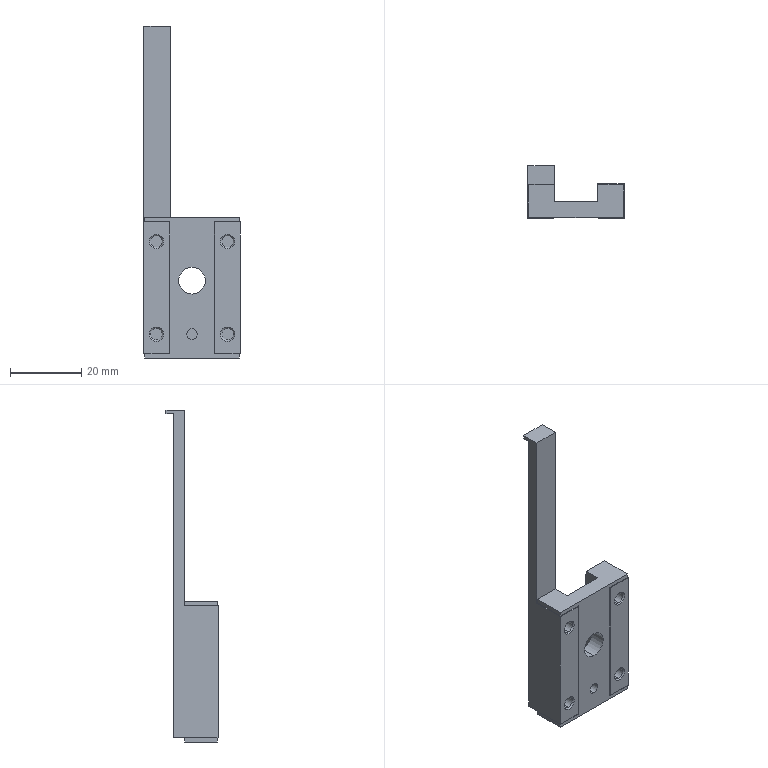Part | SolidWorks | features BaseBody 1 | 1 solid | 54 faces | box 27 x 14.6 x 93.2 mm | volume 9543 mm3 | plane 34 | cylinder 12 | cone 8 | commonest cylinder face diameters 3.242 x8 3 x2 7.5 x2
STEP:
#1=CARTESIAN_POINT('',(-10.,-32.621,-37.079));
#2=VERTEX_POINT('',#1);
#3=CARTESIAN_POINT('',(-10.,-32.621,-40.321));
#4=VERTEX_POINT('',#3);
#5=CARTESIAN_POINT('',(-10.,-32.621,-38.7));
#6=DIRECTION('',(0.,-1.,0.));
#7=DIRECTION('',(-1.,0.,0.));
#8=AXIS2_PLACEMENT_3D('',#5,#6,#7);
#9=CIRCLE('',#8,1.621);
#10=EDGE_CURVE('',#2,#4,#9,.T.);
#11=ORIENTED_EDGE('',*,*,#10,.F.);
#12=CARTESIAN_POINT('',(-10.,-33.,-36.7));
#13=VERTEX_POINT('',#12);
#14=CARTESIAN_POINT('',(-10.,-33.,-36.7));
#15=DIRECTION('',(0.,-0.7071,0.7071));
#16=VECTOR('',#15,1000.);
#17=LINE('',#14,#16);
#18=EDGE_CURVE('',#2,#13,#17,.T.);
#19=ORIENTED_EDGE('',*,*,#18,.T.);
#20=CARTESIAN_POINT('',(-10.,-33.,-40.7));
#21=VERTEX_POINT('',#20);
#22=CARTESIAN_POINT('',(-10.,-33.,-38.7));
#23=DIRECTION('',(0.,1.,0.));
#24=DIRECTION('',(0.,0.,-1.));
#25=AXIS2_PLACEMENT_3D('',#22,#23,#24);
#26=CIRCLE('',#25,2.);
#27=EDGE_CURVE('',#21,#13,#26,.T.);
#28=ORIENTED_EDGE('',*,*,#27,.F.);
#29=CARTESIAN_POINT('',(-10.,-33.,-40.7));
#30=DIRECTION('',(0.,-0.7071,-0.7071));
#31=VECTOR('',#30,1000.);
#32=LINE('',#29,#31);
#33=EDGE_CURVE('',#4,#21,#32,.T.);
#34=ORIENTED_EDGE('',*,*,#33,.F.);
#35=EDGE_LOOP('',(#11,#19,#28,#34));
#36=FACE_OUTER_BOUND('',#35,.T.);
#37=CARTESIAN_POINT('',(-10.,-33.,-38.7));
#38=DIRECTION('',(0.,-1.,0.));
#39=DIRECTION('',(0.,0.,-1.));
#40=AXIS2_PLACEMENT_3D('',#37,#38,#39);
#41=CONICAL_SURFACE('',#40,2.,0.7854);
#42=ADVANCED_FACE('',(#36),#41,.F.);
#43=CARTESIAN_POINT('',(-10.,-32.621,-63.079));
#44=VERTEX_POINT('',#43);
#45=CARTESIAN_POINT('',(-10.,-32.621,-66.321));
#46=VERTEX_POINT('',#45);
#47=CARTESIAN_POINT('',(-10.,-32.621,-64.7));
#48=DIRECTION('',(0.,-1.,0.));
#49=DIRECTION('',(-1.,0.,0.));
#50=AXIS2_PLACEMENT_3D('',#47,#48,#49);
#51=CIRCLE('',#50,1.621);
#52=EDGE_CURVE('',#44,#46,#51,.T.);
#53=ORIENTED_EDGE('',*,*,#52,.F.);
#54=CARTESIAN_POINT('',(-10.,-33.,-62.7));
#55=VERTEX_POINT('',#54);
#56=CARTESIAN_POINT('',(-10.,-33.,-62.7));
#57=DIRECTION('',(0.,-0.7071,0.7071));
#58=VECTOR('',#57,1000.);
#59=LINE('',#56,#58);
#60=EDGE_CURVE('',#44,#55,#59,.T.);
#61=ORIENTED_EDGE('',*,*,#60,.T.);
#62=CARTESIAN_POINT('',(-10.,-33.,-66.7));
#63=VERTEX_POINT('',#62);
#64=CARTESIAN_POINT('',(-10.,-33.,-64.7));
#65=DIRECTION('',(0.,1.,0.));
#66=DIRECTION('',(0.,0.,-1.));
#67=AXIS2_PLACEMENT_3D('',#64,#65,#66);
#68=CIRCLE('',#67,2.);
#69=EDGE_CURVE('',#63,#55,#68,.T.);
#70=ORIENTED_EDGE('',*,*,#69,.F.);
#71=CARTESIAN_POINT('',(-10.,-33.,-66.7));
#72=DIRECTION('',(0.,-0.7071,-0.7071));
#73=VECTOR('',#72,1000.);
#74=LINE('',#71,#73);
#75=EDGE_CURVE('',#46,#63,#74,.T.);
#76=ORIENTED_EDGE('',*,*,#75,.F.);
#77=EDGE_LOOP('',(#53,#61,#70,#76));
#78=FACE_OUTER_BOUND('',#77,.T.);
#79=CARTESIAN_POINT('',(-10.,-33.,-64.7));
#80=DIRECTION('',(0.,-1.,0.));
#81=DIRECTION('',(0.,0.,-1.));
#82=AXIS2_PLACEMENT_3D('',#79,#80,#81);
#83=CONICAL_SURFACE('',#82,2.,0.7854);
#84=ADVANCED_FACE('',(#78),#83,.F.);
#85=CARTESIAN_POINT('',(0.,-29.8,-63.2));
#86=VERTEX_POINT('',#85);
#87=CARTESIAN_POINT('',(0.,-29.8,-66.2));
#88=VERTEX_POINT('',#87);
#89=CARTESIAN_POINT('',(0.,-29.8,-64.7));
#90=DIRECTION('',(0.,-1.,0.));
#91=DIRECTION('',(0.,0.,-1.));
#92=AXIS2_PLACEMENT_3D('',#89,#90,#91);
#93=CIRCLE('',#92,1.5);
#94=EDGE_CURVE('',#86,#88,#93,.T.);
#95=ORIENTED_EDGE('',*,*,#94,.F.);
#96=CARTESIAN_POINT('',(0.,-32.8,-63.2));
#97=VERTEX_POINT('',#96);
#98=CARTESIAN_POINT('',(0.,-32.9,-63.2));
#99=DIRECTION('',(0.,-1.,0.));
#100=VECTOR('',#99,1000.);
#101=LINE('',#98,#100);
#102=EDGE_CURVE('',#86,#97,#101,.T.);
#103=ORIENTED_EDGE('',*,*,#102,.T.);
#104=CARTESIAN_POINT('',(0.,-32.8,-66.2));
#105=VERTEX_POINT('',#104);
#106=CARTESIAN_POINT('',(0.,-32.8,-64.7));
#107=DIRECTION('',(0.,1.,0.));
#108=DIRECTION('',(0.,0.,-1.));
#109=AXIS2_PLACEMENT_3D('',#106,#107,#108);
#110=CIRCLE('',#109,1.5);
#111=EDGE_CURVE('',#105,#97,#110,.T.);
#112=ORIENTED_EDGE('',*,*,#111,.F.);
#113=CARTESIAN_POINT('',(0.,-32.9,-66.2));
#114=DIRECTION('',(0.,-1.,0.));
#115=VECTOR('',#114,1000.);
#116=LINE('',#113,#115);
#117=EDGE_CURVE('',#88,#105,#116,.T.);
#118=ORIENTED_EDGE('',*,*,#117,.F.);
#119=EDGE_LOOP('',(#95,#103,#112,#118));
#120=FACE_OUTER_BOUND('',#119,.T.);
#121=CARTESIAN_POINT('',(0.,-32.9,-64.7));
#122=DIRECTION('',(0.,-1.,0.));
#123=DIRECTION('',(0.,0.,-1.));
#124=AXIS2_PLACEMENT_3D('',#121,#122,#123);
#125=CYLINDRICAL_SURFACE('',#124,1.5);
#126=ADVANCED_FACE('',(#120),#125,.F.);
#127=CARTESIAN_POINT('',(0.,-28.3,-45.95));
#128=VERTEX_POINT('',#127);
#129=CARTESIAN_POINT('',(0.,-28.3,-53.45));
#130=VERTEX_POINT('',#129);
#131=CARTESIAN_POINT('',(0.,-28.3,-49.7));
#132=DIRECTION('',(0.,-1.,0.));
#133=DIRECTION('',(0.,0.,-1.));
#134=AXIS2_PLACEMENT_3D('',#131,#132,#133);
#135=CIRCLE('',#134,3.75);
#136=EDGE_CURVE('',#128,#130,#135,.T.);
#137=ORIENTED_EDGE('',*,*,#136,.F.);
#138=CARTESIAN_POINT('',(0.,-32.8,-45.95));
#139=VERTEX_POINT('',#138);
#140=CARTESIAN_POINT('',(0.,-32.9,-45.95));
#141=DIRECTION('',(0.,-1.,0.));
#142=VECTOR('',#141,1000.);
#143=LINE('',#140,#142);
#144=EDGE_CURVE('',#128,#139,#143,.T.);
#145=ORIENTED_EDGE('',*,*,#144,.T.);
#146=CARTESIAN_POINT('',(0.,-32.8,-53.45));
#147=VERTEX_POINT('',#146);
#148=CARTESIAN_POINT('',(0.,-32.8,-49.7));
#149=DIRECTION('',(0.,1.,0.));
#150=DIRECTION('',(0.,0.,-1.));
#151=AXIS2_PLACEMENT_3D('',#148,#149,#150);
#152=CIRCLE('',#151,3.75);
#153=EDGE_CURVE('',#147,#139,#152,.T.);
#154=ORIENTED_EDGE('',*,*,#153,.F.);
#155=CARTESIAN_POINT('',(0.,-32.9,-53.45));
#156=DIRECTION('',(0.,-1.,0.));
#157=VECTOR('',#156,1000.);
#158=LINE('',#155,#157);
#159=EDGE_CURVE('',#130,#147,#158,.T.);
#160=ORIENTED_EDGE('',*,*,#159,.F.);
#161=EDGE_LOOP('',(#137,#145,#154,#160));
#162=FACE_OUTER_BOUND('',#161,.T.);
#163=CARTESIAN_POINT('',(0.,-32.9,-49.7));
#164=DIRECTION('',(0.,-1.,0.));
#165=DIRECTION('',(0.,0.,-1.));
#166=AXIS2_PLACEMENT_3D('',#163,#164,#165);
#167=CYLINDRICAL_SURFACE('',#166,3.75);
#168=ADVANCED_FACE('',(#162),#167,.F.);
#169=CARTESIAN_POINT('',(-10.,-29.,-37.079));
#170=VERTEX_POINT('',#169);
#171=CARTESIAN_POINT('',(-10.,-29.,-40.321));
#172=VERTEX_POINT('',#171);
#173=CARTESIAN_POINT('',(-10.,-29.,-38.7));
#174=DIRECTION('',(0.,-1.,0.));
#175=DIRECTION('',(0.,0.,-1.));
#176=AXIS2_PLACEMENT_3D('',#173,#174,#175);
#177=CIRCLE('',#176,1.621);
#178=EDGE_CURVE('',#170,#172,#177,.T.);
#179=ORIENTED_EDGE('',*,*,#178,.F.);
#180=CARTESIAN_POINT('',(-10.,-30.811,-37.079));
#181=DIRECTION('',(0.,-1.,0.));
#182=VECTOR('',#181,1000.);
#183=LINE('',#180,#182);
#184=EDGE_CURVE('',#170,#2,#183,.T.);
#185=ORIENTED_EDGE('',*,*,#184,.T.);
#186=ORIENTED_EDGE('',*,*,#10,.T.);
#187=CARTESIAN_POINT('',(-10.,-30.811,-40.321));
#188=DIRECTION('',(0.,-1.,0.));
#189=VECTOR('',#188,1000.);
#190=LINE('',#187,#189);
#191=EDGE_CURVE('',#172,#4,#190,.T.);
#192=ORIENTED_EDGE('',*,*,#191,.F.);
#193=EDGE_LOOP('',(#179,#185,#186,#192));
#194=FACE_OUTER_BOUND('',#193,.T.);
#195=CARTESIAN_POINT('',(-10.,-30.811,-38.7));
#196=DIRECTION('',(0.,-1.,0.));
#197=DIRECTION('',(0.,0.,-1.));
#198=AXIS2_PLACEMENT_3D('',#195,#196,#197);
#199=CYLINDRICAL_SURFACE('',#198,1.621);
#200=ADVANCED_FACE('',(#194),#199,.F.);
#201=CARTESIAN_POINT('',(-10.,-29.,-63.079));
#202=VERTEX_POINT('',#201);
#203=CARTESIAN_POINT('',(-10.,-29.,-66.321));
#204=VERTEX_POINT('',#203);
#205=CARTESIAN_POINT('',(-10.,-29.,-64.7));
#206=DIRECTION('',(0.,-1.,0.));
#207=DIRECTION('',(0.,0.,-1.));
#208=AXIS2_PLACEMENT_3D('',#205,#206,#207);
#209=CIRCLE('',#208,1.621);
#210=EDGE_CURVE('',#202,#204,#209,.T.);
#211=ORIENTED_EDGE('',*,*,#210,.F.);
#212=CARTESIAN_POINT('',(-10.,-30.811,-63.079));
#213=DIRECTION('',(0.,-1.,0.));
#214=VECTOR('',#213,1000.);
#215=LINE('',#212,#214);
#216=EDGE_CURVE('',#202,#44,#215,.T.);
#217=ORIENTED_EDGE('',*,*,#216,.T.);
#218=ORIENTED_EDGE('',*,*,#52,.T.);
#219=CARTESIAN_POINT('',(-10.,-30.811,-66.321));
#220=DIRECTION('',(0.,-1.,0.));
#221=VECTOR('',#220,1000.);
#222=LINE('',#219,#221);
#223=EDGE_CURVE('',#204,#46,#222,.T.);
#224=ORIENTED_EDGE('',*,*,#223,.F.);
#225=EDGE_LOOP('',(#211,#217,#218,#224));
#226=FACE_OUTER_BOUND('',#225,.T.);
#227=CARTESIAN_POINT('',(-10.,-30.811,-64.7));
#228=DIRECTION('',(0.,-1.,0.));
#229=DIRECTION('',(0.,0.,-1.));
#230=AXIS2_PLACEMENT_3D('',#227,#228,#229);
#231=CYLINDRICAL_SURFACE('',#230,1.621);
#232=ADVANCED_FACE('',(#226),#231,.F.);
#233=CARTESIAN_POINT('',(10.,-32.621,-37.079));
#234=VERTEX_POINT('',#233);
#235=CARTESIAN_POINT('',(10.,-32.621,-40.321));
#236=VERTEX_POINT('',#235);
#237=CARTESIAN_POINT('',(10.,-32.621,-38.7));
#238=DIRECTION('',(0.,-1.,0.));
#239=DIRECTION('',(-1.,0.,0.));
#240=AXIS2_PLACEMENT_3D('',#237,#238,#239);
#241=CIRCLE('',#240,1.621);
#242=EDGE_CURVE('',#234,#236,#241,.T.);
#243=ORIENTED_EDGE('',*,*,#242,.F.);
#244=CARTESIAN_POINT('',(10.,-33.,-36.7));
#245=VERTEX_POINT('',#244);
#246=CARTESIAN_POINT('',(10.,-33.,-36.7));
#247=DIRECTION('',(0.,-0.7071,0.7071));
#248=VECTOR('',#247,1000.);
#249=LINE('',#246,#248);
#250=EDGE_CURVE('',#234,#245,#249,.T.);
#251=ORIENTED_EDGE('',*,*,#250,.T.);
#252=CARTESIAN_POINT('',(10.,-33.,-40.7));
#253=VERTEX_POINT('',#252);
#254=CARTESIAN_POINT('',(10.,-33.,-38.7));
#255=DIRECTION('',(0.,1.,0.));
#256=DIRECTION('',(0.,0.,-1.));
#257=AXIS2_PLACEMENT_3D('',#254,#255,#256);
#258=CIRCLE('',#257,2.);
#259=EDGE_CURVE('',#253,#245,#258,.T.);
#260=ORIENTED_EDGE('',*,*,#259,.F.);
#261=CARTESIAN_POINT('',(10.,-33.,-40.7));
#262=DIRECTION('',(0.,-0.7071,-0.7071));
#263=VECTOR('',#262,1000.);
#264=LINE('',#261,#263);
#265=EDGE_CURVE('',#236,#253,#264,.T.);
#266=ORIENTED_EDGE('',*,*,#265,.F.);
#267=EDGE_LOOP('',(#243,#251,#260,#266));
#268=FACE_OUTER_BOUND('',#267,.T.);
#269=CARTESIAN_POINT('',(10.,-33.,-38.7));
#270=DIRECTION('',(0.,-1.,0.));
#271=DIRECTION('',(0.,0.,-1.));
#272=AXIS2_PLACEMENT_3D('',#269,#270,#271);
#273=CONICAL_SURFACE('',#272,2.,0.7854);
#274=ADVANCED_FACE('',(#268),#273,.F.);
#275=CARTESIAN_POINT('',(10.,-32.621,-63.079));
#276=VERTEX_POINT('',#275);
#277=CARTESIAN_POINT('',(10.,-32.621,-66.321));
#278=VERTEX_POINT('',#277);
#279=CARTESIAN_POINT('',(10.,-32.621,-64.7));
#280=DIRECTION('',(0.,-1.,0.));
#281=DIRECTION('',(-1.,0.,0.));
#282=AXIS2_PLACEMENT_3D('',#279,#280,#281);
#283=CIRCLE('',#282,1.621);
#284=EDGE_CURVE('',#276,#278,#283,.T.);
#285=ORIENTED_EDGE('',*,*,#284,.F.);
#286=CARTESIAN_POINT('',(10.,-33.,-62.7));
#287=VERTEX_POINT('',#286);
#288=CARTESIAN_POINT('',(10.,-33.,-62.7));
#289=DIRECTION('',(0.,-0.7071,0.7071));
#290=VECTOR('',#289,1000.);
#291=LINE('',#288,#290);
#292=EDGE_CURVE('',#276,#287,#291,.T.);
#293=ORIENTED_EDGE('',*,*,#292,.T.);
#294=CARTESIAN_POINT('',(10.,-33.,-66.7));
#295=VERTEX_POINT('',#294);
#296=CARTESIAN_POINT('',(10.,-33.,-64.7));
#297=DIRECTION('',(0.,1.,0.));
#298=DIRECTION('',(0.,0.,-1.));
#299=AXIS2_PLACEMENT_3D('',#296,#297,#298);
#300=CIRCLE('',#299,2.);
#301=EDGE_CURVE('',#295,#287,#300,.T.);
#302=ORIENTED_EDGE('',*,*,#301,.F.);
#303=CARTESIAN_POINT('',(10.,-33.,-66.7));
#304=DIRECTION('',(0.,-0.7071,-0.7071));
#305=VECTOR('',#304,1000.);
#306=LINE('',#303,#305);
#307=EDGE_CURVE('',#278,#295,#306,.T.);
#308=ORIENTED_EDGE('',*,*,#307,.F.);
#309=EDGE_LOOP('',(#285,#293,#302,#308));
#310=FACE_OUTER_BOUND('',#309,.T.);
#311=CARTESIAN_POINT('',(10.,-33.,-64.7));
#312=DIRECTION('',(0.,-1.,0.));
#313=DIRECTION('',(0.,0.,-1.));
#314=AXIS2_PLACEMENT_3D('',#311,#312,#313);
#315=CONICAL_SURFACE('',#314,2.,0.7854);
#316=ADVANCED_FACE('',(#310),#315,.F.);
#317=CARTESIAN_POINT('',(10.,-29.,-37.079));
#318=VERTEX_POINT('',#317);
#319=CARTESIAN_POINT('',(10.,-29.,-40.321));
#320=VERTEX_POINT('',#319);
#321=CARTESIAN_POINT('',(10.,-29.,-38.7));
#322=DIRECTION('',(0.,-1.,0.));
#323=DIRECTION('',(0.,0.,-1.));
#324=AXIS2_PLACEMENT_3D('',#321,#322,#323);
#325=CIRCLE('',#324,1.621);
#326=EDGE_CURVE('',#318,#320,#325,.T.);
#327=ORIENTED_EDGE('',*,*,#326,.F.);
#328=CARTESIAN_POINT('',(10.,-30.811,-37.079));
#329=DIRECTION('',(0.,-1.,0.));
#330=VECTOR('',#329,1000.);
#331=LINE('',#328,#330);
#332=EDGE_CURVE('',#318,#234,#331,.T.);
#333=ORIENTED_EDGE('',*,*,#332,.T.);
#334=ORIENTED_EDGE('',*,*,#242,.T.);
#335=CARTESIAN_POINT('',(10.,-30.811,-40.321));
#336=DIRECTION('',(0.,-1.,0.));
#337=VECTOR('',#336,1000.);
#338=LINE('',#335,#337);
#339=EDGE_CURVE('',#320,#236,#338,.T.);
#340=ORIENTED_EDGE('',*,*,#339,.F.);
#341=EDGE_LOOP('',(#327,#333,#334,#340));
#342=FACE_OUTER_BOUND('',#341,.T.);
#343=CARTESIAN_POINT('',(10.,-30.811,-38.7));
#344=DIRECTION('',(0.,-1.,0.));
#345=DIRECTION('',(0.,0.,-1.));
#346=AXIS2_PLACEMENT_3D('',#343,#344,#345);
#347=CYLINDRICAL_SURFACE('',#346,1.621);
#348=ADVANCED_FACE('',(#342),#347,.F.);
#349=CARTESIAN_POINT('',(10.,-29.,-63.079));
#350=VERTEX_POINT('',#349);
#351=CARTESIAN_POINT('',(10.,-29.,-66.321));
#352=VERTEX_POINT('',#351);
#353=CARTESIAN_POINT('',(10.,-29.,-64.7));
#354=DIRECTION('',(0.,-1.,0.));
#355=DIRECTION('',(0.,0.,-1.));
#356=AXIS2_PLACEMENT_3D('',#353,#354,#355);
#357=CIRCLE('',#356,1.621);
#358=EDGE_CURVE('',#350,#352,#357,.T.);
#359=ORIENTED_EDGE('',*,*,#358,.F.);
#360=CARTESIAN_POINT('',(10.,-30.811,-63.079));
#361=DIRECTION('',(0.,-1.,0.));
#362=VECTOR('',#361,1000.);
#363=LINE('',#360,#362);
#364=EDGE_CURVE('',#350,#276,#363,.T.);
#365=ORIENTED_EDGE('',*,*,#364,.T.);
#366=ORIENTED_EDGE('',*,*,#284,.T.);
#367=CARTESIAN_POINT('',(10.,-30.811,-66.321));
#368=DIRECTION('',(0.,-1.,0.));
#369=VECTOR('',#368,1000.);
#370=LINE('',#367,#369);
#371=EDGE_CURVE('',#352,#278,#370,.T.);
#372=ORIENTED_EDGE('',*,*,#371,.F.);
#373=EDGE_LOOP('',(#359,#365,#366,#372));
#374=FACE_OUTER_BOUND('',#373,.T.);
#375=CARTESIAN_POINT('',(10.,-30.811,-64.7));
#376=DIRECTION('',(0.,-1.,0.));
#377=DIRECTION('',(0.,0.,-1.));
#378=AXIS2_PLACEMENT_3D('',#375,#376,#377);
#379=CYLINDRICAL_SURFACE('',#378,1.621);
#380=ADVANCED_FACE('',(#374),#379,.F.);
#381=CARTESIAN_POINT('',(-6.1,-20.4,-70.2));
#382=VERTEX_POINT('',#381);
#383=CARTESIAN_POINT('',(-13.5,-20.4,-70.2));
#384=VERTEX_POINT('',#383);
#385=CARTESIAN_POINT('',(-6.1,-20.4,-70.2));
#386=DIRECTION('',(-1.,0.,0.));
#387=VECTOR('',#386,1000.);
#388=LINE('',#385,#387);
#389=EDGE_CURVE('',#382,#384,#388,.T.);
#390=ORIENTED_EDGE('',*,*,#389,.T.);
#391=CARTESIAN_POINT('',(-13.5,-20.4,20.8));
#392=VERTEX_POINT('',#391);
#393=CARTESIAN_POINT('',(-13.5,-20.4,-32.));
#394=DIRECTION('',(0.,0.,1.));
#395=VECTOR('',#394,1000.);
#396=LINE('',#393,#395);
#397=EDGE_CURVE('',#384,#392,#396,.T.);
#398=ORIENTED_EDGE('',*,*,#397,.T.);
#399=CARTESIAN_POINT('',(-6.1,-20.4,20.8));
#400=VERTEX_POINT('',#399);
#401=CARTESIAN_POINT('',(-6.1,-20.4,20.8));
#402=DIRECTION('',(1.,0.,0.));
#403=VECTOR('',#402,1000.);
#404=LINE('',#401,#403);
#405=EDGE_CURVE('',#392,#400,#404,.T.);
#406=ORIENTED_EDGE('',*,*,#405,.T.);
#407=CARTESIAN_POINT('',(-6.1,-20.4,-32.));
#408=DIRECTION('',(0.,0.,-1.));
#409=VECTOR('',#408,1000.);
#410=LINE('',#407,#409);
#411=EDGE_CURVE('',#400,#382,#410,.T.);
#412=ORIENTED_EDGE('',*,*,#411,.T.);
#413=EDGE_LOOP('',(#390,#398,#406,#412));
#414=FACE_OUTER_BOUND('',#413,.T.);
#415=CARTESIAN_POINT('',(-6.1,-20.4,-32.));
#416=DIRECTION('',(0.,1.,0.));
#417=DIRECTION('',(-1.,0.,0.));
#418=AXIS2_PLACEMENT_3D('',#415,#416,#417);
#419=PLANE('',#418);
#420=ADVANCED_FACE('',(#414),#419,.T.);
#421=CARTESIAN_POINT('',(-13.5,-18.4,20.8));
#422=VERTEX_POINT('',#421);
#423=CARTESIAN_POINT('',(-13.5,-20.4,20.8));
#424=DIRECTION('',(0.,-1.,0.));
#425=VECTOR('',#424,1000.);
#426=LINE('',#423,#425);
#427=EDGE_CURVE('',#422,#392,#426,.T.);
#428=ORIENTED_EDGE('',*,*,#427,.T.);
#429=ORIENTED_EDGE('',*,*,#397,.F.);
#430=CARTESIAN_POINT('',(-13.5,-33.,-70.2));
#431=VERTEX_POINT('',#430);
#432=CARTESIAN_POINT('',(-13.5,-20.4,-70.2));
#433=DIRECTION('',(0.,-1.,0.));
#434=VECTOR('',#433,1000.);
#435=LINE('',#432,#434);
#436=EDGE_CURVE('',#384,#431,#435,.T.);
#437=ORIENTED_EDGE('',*,*,#436,.T.);
#438=CARTESIAN_POINT('',(-13.5,-33.,-33.2));
#439=VERTEX_POINT('',#438);
#440=CARTESIAN_POINT('',(-13.5,-33.,-32.));
#441=DIRECTION('',(0.,0.,1.));
#442=VECTOR('',#441,1000.);
#443=LINE('',#440,#442);
#444=EDGE_CURVE('',#431,#439,#443,.T.);
#445=ORIENTED_EDGE('',*,*,#444,.T.);
#446=CARTESIAN_POINT('',(-13.5,-23.6,-33.2));
#447=VERTEX_POINT('',#446);
#448=CARTESIAN_POINT('',(-13.5,-20.4,-33.2));
#449=DIRECTION('',(0.,1.,0.));
#450=VECTOR('',#449,1000.);
#451=LINE('',#448,#450);
#452=EDGE_CURVE('',#439,#447,#451,.T.);
#453=ORIENTED_EDGE('',*,*,#452,.T.);
#454=CARTESIAN_POINT('',(-13.5,-23.6,21.8));
#455=VERTEX_POINT('',#454);
#456=CARTESIAN_POINT('',(-13.5,-23.6,-32.));
#457=DIRECTION('',(0.,0.,1.));
#458=VECTOR('',#457,1000.);
#459=LINE('',#456,#458);
#460=EDGE_CURVE('',#447,#455,#459,.T.);
#461=ORIENTED_EDGE('',*,*,#460,.T.);
#462=CARTESIAN_POINT('',(-13.5,-18.4,21.8));
#463=VERTEX_POINT('',#462);
#464=CARTESIAN_POINT('',(-13.5,-20.4,21.8));
#465=DIRECTION('',(0.,1.,0.));
#466=VECTOR('',#465,1000.);
#467=LINE('',#464,#466);
#468=EDGE_CURVE('',#455,#463,#467,.T.);
#469=ORIENTED_EDGE('',*,*,#468,.T.);
#470=CARTESIAN_POINT('',(-13.5,-18.4,21.8));
#471=DIRECTION('',(0.,0.,1.));
#472=VECTOR('',#471,1000.);
#473=LINE('',#470,#472);
#474=EDGE_CURVE('',#422,#463,#473,.T.);
#475=ORIENTED_EDGE('',*,*,#474,.F.);
#476=EDGE_LOOP('',(#428,#429,#437,#445,#453,#461,#469,#475));
#477=FACE_OUTER_BOUND('',#476,.T.);
#478=CARTESIAN_POINT('',(-13.5,-20.4,-32.));
#479=DIRECTION('',(-1.,0.,0.));
#480=DIRECTION('',(0.,0.,1.));
#481=AXIS2_PLACEMENT_3D('',#478,#479,#480);
#482=PLANE('',#481);
#483=ADVANCED_FACE('',(#477),#482,.T.);
#484=CARTESIAN_POINT('',(-13.3,-23.7,-70.2));
#485=VERTEX_POINT('',#484);
#486=CARTESIAN_POINT('',(-13.3,-32.8,-70.2));
#487=VERTEX_POINT('',#486);
#488=CARTESIAN_POINT('',(-13.3,-33.,-70.2));
#489=DIRECTION('',(0.,-1.,0.));
#490=VECTOR('',#489,1000.);
#491=LINE('',#488,#490);
#492=EDGE_CURVE('',#485,#487,#491,.T.);
#493=ORIENTED_EDGE('',*,*,#492,.T.);
#494=CARTESIAN_POINT('',(-6.2,-32.8,-70.2));
#495=VERTEX_POINT('',#494);
#496=CARTESIAN_POINT('',(0.,-32.8,-70.2));
#497=DIRECTION('',(1.,0.,0.));
#498=VECTOR('',#497,1000.);
#499=LINE('',#496,#498);
#500=EDGE_CURVE('',#487,#495,#499,.T.);
#501=ORIENTED_EDGE('',*,*,#500,.T.);
#502=CARTESIAN_POINT('',(-6.4,-33.,-70.2));
#503=VERTEX_POINT('',#502);
#504=CARTESIAN_POINT('',(-6.4,-33.,-70.2));
#505=DIRECTION('',(0.7071,0.7071,0.));
#506=VECTOR('',#505,1000.);
#507=LINE('',#504,#506);
#508=EDGE_CURVE('',#503,#495,#507,.T.);
#509=ORIENTED_EDGE('',*,*,#508,.F.);
#510=CARTESIAN_POINT('',(0.,-33.,-70.2));
#511=DIRECTION('',(-1.,0.,0.));
#512=VECTOR('',#511,1000.);
#513=LINE('',#510,#512);
#514=EDGE_CURVE('',#503,#431,#513,.T.);
#515=ORIENTED_EDGE('',*,*,#514,.T.);
#516=ORIENTED_EDGE('',*,*,#436,.F.);
#517=ORIENTED_EDGE('',*,*,#389,.F.);
#518=CARTESIAN_POINT('',(-6.1,-23.7,-70.2));
#519=VERTEX_POINT('',#518);
#520=CARTESIAN_POINT('',(-6.1,-33.,-70.2));
#521=DIRECTION('',(0.,-1.,0.));
#522=VECTOR('',#521,1000.);
#523=LINE('',#520,#522);
#524=EDGE_CURVE('',#382,#519,#523,.T.);
#525=ORIENTED_EDGE('',*,*,#524,.T.);
#526=CARTESIAN_POINT('',(0.,-23.7,-70.2));
#527=DIRECTION('',(-1.,0.,0.));
#528=VECTOR('',#527,1000.);
#529=LINE('',#526,#528);
#530=EDGE_CURVE('',#519,#485,#529,.T.);
#531=ORIENTED_EDGE('',*,*,#530,.T.);
#532=EDGE_LOOP('',(#493,#501,#509,#515,#516,#517,#525,#531));
#533=FACE_OUTER_BOUND('',#532,.T.);
#534=CARTESIAN_POINT('',(0.,-33.,-70.2));
#535=DIRECTION('',(0.,0.,-1.));
#536=DIRECTION('',(-1.,0.,0.));
#537=AXIS2_PLACEMENT_3D('',#534,#535,#536);
#538=PLANE('',#537);
#539=ADVANCED_FACE('',(#533),#538,.T.);
#540=CARTESIAN_POINT('',(-6.1,-18.4,20.8));
#541=VERTEX_POINT('',#540);
#542=CARTESIAN_POINT('',(-6.1,-28.3,20.8));
#543=DIRECTION('',(0.,1.,0.));
#544=VECTOR('',#543,1000.);
#545=LINE('',#542,#544);
#546=EDGE_CURVE('',#400,#541,#545,.T.);
#547=ORIENTED_EDGE('',*,*,#546,.T.);
#548=CARTESIAN_POINT('',(-6.1,-18.4,21.8));
#549=VERTEX_POINT('',#548);
#550=CARTESIAN_POINT('',(-6.1,-18.4,21.8));
#551=DIRECTION('',(0.,0.,-1.));
#552=VECTOR('',#551,1000.);
#553=LINE('',#550,#552);
#554=EDGE_CURVE('',#549,#541,#553,.T.);
#555=ORIENTED_EDGE('',*,*,#554,.F.);
#556=CARTESIAN_POINT('',(-6.1,-23.6,21.8));
#557=VERTEX_POINT('',#556);
#558=CARTESIAN_POINT('',(-6.1,-28.3,21.8));
#559=DIRECTION('',(0.,-1.,0.));
#560=VECTOR('',#559,1000.);
#561=LINE('',#558,#560);
#562=EDGE_CURVE('',#549,#557,#561,.T.);
#563=ORIENTED_EDGE('',*,*,#562,.T.);
#564=CARTESIAN_POINT('',(-6.1,-23.6,-32.));
#565=VERTEX_POINT('',#564);
#566=CARTESIAN_POINT('',(-6.1,-23.6,-32.));
#567=DIRECTION('',(0.,0.,-1.));
#568=VECTOR('',#567,1000.);
#569=LINE('',#566,#568);
#570=EDGE_CURVE('',#557,#565,#569,.T.);
#571=ORIENTED_EDGE('',*,*,#570,.T.);
#572=CARTESIAN_POINT('',(-6.1,-28.3,-32.));
#573=VERTEX_POINT('',#572);
#574=CARTESIAN_POINT('',(-6.1,-28.3,-32.));
#575=DIRECTION('',(0.,-1.,0.));
#576=VECTOR('',#575,1000.);
#577=LINE('',#574,#576);
#578=EDGE_CURVE('',#565,#573,#577,.T.);
#579=ORIENTED_EDGE('',*,*,#578,.T.);
#580=CARTESIAN_POINT('',(-6.1,-28.3,-71.4));
#581=VERTEX_POINT('',#580);
#582=CARTESIAN_POINT('',(-6.1,-28.3,-32.));
#583=DIRECTION('',(0.,0.,-1.));
#584=VECTOR('',#583,1000.);
#585=LINE('',#582,#584);
#586=EDGE_CURVE('',#573,#581,#585,.T.);
#587=ORIENTED_EDGE('',*,*,#586,.T.);
#588=CARTESIAN_POINT('',(-6.1,-23.7,-71.4));
#589=VERTEX_POINT('',#588);
#590=CARTESIAN_POINT('',(-6.1,-28.3,-71.4));
#591=DIRECTION('',(0.,1.,0.));
#592=VECTOR('',#591,1000.);
#593=LINE('',#590,#592);
#594=EDGE_CURVE('',#581,#589,#593,.T.);
#595=ORIENTED_EDGE('',*,*,#594,.T.);
#596=CARTESIAN_POINT('',(-6.1,-23.7,-32.));
#597=DIRECTION('',(0.,0.,1.));
#598=VECTOR('',#597,1000.);
#599=LINE('',#596,#598);
#600=EDGE_CURVE('',#589,#519,#599,.T.);
#601=ORIENTED_EDGE('',*,*,#600,.T.);
#602=ORIENTED_EDGE('',*,*,#524,.F.);
#603=ORIENTED_EDGE('',*,*,#411,.F.);
#604=EDGE_LOOP('',(#547,#555,#563,#571,#579,#587,#595,#601,#602,#603));
#605=FACE_OUTER_BOUND('',#604,.T.);
#606=CARTESIAN_POINT('',(-6.1,-28.3,-32.));
#607=DIRECTION('',(1.,0.,0.));
#608=DIRECTION('',(0.,1.,0.));
#609=AXIS2_PLACEMENT_3D('',#606,#607,#608);
#610=PLANE('',#609);
#611=ADVANCED_FACE('',(#605),#610,.T.);
#612=ORIENTED_EDGE('',*,*,#427,.F.);
#613=CARTESIAN_POINT('',(0.,-18.4,20.8));
#614=DIRECTION('',(1.,0.,0.));
#615=VECTOR('',#614,1000.);
#616=LINE('',#613,#615);
#617=EDGE_CURVE('',#422,#541,#616,.T.);
#618=ORIENTED_EDGE('',*,*,#617,.T.);
#619=ORIENTED_EDGE('',*,*,#546,.F.);
#620=ORIENTED_EDGE('',*,*,#405,.F.);
#621=EDGE_LOOP('',(#612,#618,#619,#620));
#622=FACE_OUTER_BOUND('',#621,.T.);
#623=CARTESIAN_POINT('',(0.,-33.,20.8));
#624=DIRECTION('',(0.,0.,-1.));
#625=DIRECTION('',(-1.,0.,0.));
#626=AXIS2_PLACEMENT_3D('',#623,#624,#625);
#627=PLANE('',#626);
#628=ADVANCED_FACE('',(#622),#627,.T.);
#629=CARTESIAN_POINT('',(0.,-23.6,21.8));
#630=DIRECTION('',(-1.,0.,0.));
#631=VECTOR('',#630,1000.);
#632=LINE('',#629,#631);
#633=EDGE_CURVE('',#557,#455,#632,.T.);
#634=ORIENTED_EDGE('',*,*,#633,.F.);
#635=ORIENTED_EDGE('',*,*,#562,.F.);
#636=CARTESIAN_POINT('',(0.,-18.4,21.8));
#637=DIRECTION('',(1.,0.,0.));
#638=VECTOR('',#637,1000.);
#639=LINE('',#636,#638);
#640=EDGE_CURVE('',#463,#549,#639,.T.);
#641=ORIENTED_EDGE('',*,*,#640,.F.);
#642=ORIENTED_EDGE('',*,*,#468,.F.);
#643=EDGE_LOOP('',(#634,#635,#641,#642));
#644=FACE_OUTER_BOUND('',#643,.T.);
#645=CARTESIAN_POINT('',(0.,-33.,21.8));
#646=DIRECTION('',(0.,0.,-1.));
#647=DIRECTION('',(-1.,0.,0.));
#648=AXIS2_PLACEMENT_3D('',#645,#646,#647);
#649=PLANE('',#648);
#650=ADVANCED_FACE('',(#644),#649,.F.);
#651=CARTESIAN_POINT('',(-13.3,-23.6,-33.2));
#652=VERTEX_POINT('',#651);
#653=CARTESIAN_POINT('',(-6.1,-23.6,-33.2));
#654=DIRECTION('',(1.,0.,0.));
#655=VECTOR('',#654,1000.);
#656=LINE('',#653,#655);
#657=EDGE_CURVE('',#447,#652,#656,.T.);
#658=ORIENTED_EDGE('',*,*,#657,.T.);
#659=CARTESIAN_POINT('',(-13.3,-23.6,-32.));
#660=VERTEX_POINT('',#659);
#661=CARTESIAN_POINT('',(-13.3,-23.6,-32.));
#662=DIRECTION('',(0.,0.,1.));
#663=VECTOR('',#662,1000.);
#664=LINE('',#661,#663);
#665=EDGE_CURVE('',#652,#660,#664,.T.);
#666=ORIENTED_EDGE('',*,*,#665,.T.);
#667=CARTESIAN_POINT('',(-6.1,-23.6,-32.));
#668=DIRECTION('',(1.,0.,0.));
#669=VECTOR('',#668,1000.);
#670=LINE('',#667,#669);
#671=EDGE_CURVE('',#660,#565,#670,.T.);
#672=ORIENTED_EDGE('',*,*,#671,.T.);
#673=ORIENTED_EDGE('',*,*,#570,.F.);
#674=ORIENTED_EDGE('',*,*,#633,.T.);
#675=ORIENTED_EDGE('',*,*,#460,.F.);
#676=EDGE_LOOP('',(#658,#666,#672,#673,#674,#675));
#677=FACE_OUTER_BOUND('',#676,.T.);
#678=CARTESIAN_POINT('',(-6.1,-23.6,-33.2));
#679=DIRECTION('',(0.,-1.,0.));
#680=DIRECTION('',(0.,0.,-1.));
#681=AXIS2_PLACEMENT_3D('',#678,#679,#680);
#682=PLANE('',#681);
#683=ADVANCED_FACE('',(#677),#682,.T.);
#684=ORIENTED_EDGE('',*,*,#452,.F.);
#685=CARTESIAN_POINT('',(-6.4,-33.,-33.2));
#686=VERTEX_POINT('',#685);
#687=CARTESIAN_POINT('',(0.,-33.,-33.2));
#688=DIRECTION('',(-1.,0.,0.));
#689=VECTOR('',#688,1000.);
#690=LINE('',#687,#689);
#691=EDGE_CURVE('',#686,#439,#690,.T.);
#692=ORIENTED_EDGE('',*,*,#691,.F.);
#693=CARTESIAN_POINT('',(-6.2,-32.8,-33.2));
#694=VERTEX_POINT('',#693);
#695=CARTESIAN_POINT('',(-6.4,-33.,-33.2));
#696=DIRECTION('',(-0.7071,-0.7071,0.));
#697=VECTOR('',#696,1000.);
#698=LINE('',#695,#697);
#699=EDGE_CURVE('',#694,#686,#698,.T.);
#700=ORIENTED_EDGE('',*,*,#699,.F.);
#701=CARTESIAN_POINT('',(-13.3,-32.8,-33.2));
#702=VERTEX_POINT('',#701);
#703=CARTESIAN_POINT('',(0.,-32.8,-33.2));
#704=DIRECTION('',(1.,0.,0.));
#705=VECTOR('',#704,1000.);
#706=LINE('',#703,#705);
#707=EDGE_CURVE('',#702,#694,#706,.T.);
#708=ORIENTED_EDGE('',*,*,#707,.F.);
#709=CARTESIAN_POINT('',(-13.3,-33.,-33.2));
#710=DIRECTION('',(0.,-1.,0.));
#711=VECTOR('',#710,1000.);
#712=LINE('',#709,#711);
#713=EDGE_CURVE('',#652,#702,#712,.T.);
#714=ORIENTED_EDGE('',*,*,#713,.F.);
#715=ORIENTED_EDGE('',*,*,#657,.F.);
#716=EDGE_LOOP('',(#684,#692,#700,#708,#714,#715));
#717=FACE_OUTER_BOUND('',#716,.T.);
#718=CARTESIAN_POINT('',(0.,-33.,-33.2));
#719=DIRECTION('',(0.,0.,-1.));
#720=DIRECTION('',(-1.,0.,0.));
#721=AXIS2_PLACEMENT_3D('',#718,#719,#720);
#722=PLANE('',#721);
#723=ADVANCED_FACE('',(#717),#722,.F.);
#724=ORIENTED_EDGE('',*,*,#691,.T.);
#725=ORIENTED_EDGE('',*,*,#444,.F.);
#726=ORIENTED_EDGE('',*,*,#514,.F.);
#727=CARTESIAN_POINT('',(-6.4,-33.,-32.));
#728=DIRECTION('',(0.,0.,1.));
#729=VECTOR('',#728,1000.);
#730=LINE('',#727,#729);
#731=EDGE_CURVE('',#503,#686,#730,.T.);
#732=ORIENTED_EDGE('',*,*,#731,.T.);
#733=EDGE_LOOP('',(#724,#725,#726,#732));
#734=FACE_OUTER_BOUND('',#733,.T.);
#735=ORIENTED_EDGE('',*,*,#27,.T.);
#736=CARTESIAN_POINT('',(-10.,-33.,-38.7));
#737=DIRECTION('',(0.,1.,0.));
#738=DIRECTION('',(0.,0.,-1.));
#739=AXIS2_PLACEMENT_3D('',#736,#737,#738);
#740=CIRCLE('',#739,2.);
#741=EDGE_CURVE('',#13,#21,#740,.T.);
#742=ORIENTED_EDGE('',*,*,#741,.T.);
#743=EDGE_LOOP('',(#735,#742));
#744=FACE_BOUND('',#743,.T.);
#745=ORIENTED_EDGE('',*,*,#69,.T.);
#746=CARTESIAN_POINT('',(-10.,-33.,-64.7));
#747=DIRECTION('',(0.,1.,0.));
#748=DIRECTION('',(0.,0.,-1.));
#749=AXIS2_PLACEMENT_3D('',#746,#747,#748);
#750=CIRCLE('',#749,2.);
#751=EDGE_CURVE('',#55,#63,#750,.T.);
#752=ORIENTED_EDGE('',*,*,#751,.T.);
#753=EDGE_LOOP('',(#745,#752));
#754=FACE_BOUND('',#753,.T.);
#755=CARTESIAN_POINT('',(-13.5,-33.,-32.));
#756=DIRECTION('',(0.,-1.,0.));
#757=DIRECTION('',(0.,0.,-1.));
#758=AXIS2_PLACEMENT_3D('',#755,#756,#757);
#759=PLANE('',#758);
#760=ADVANCED_FACE('',(#734,#744,#754),#759,.T.);
#761=CARTESIAN_POINT('',(13.3,-32.8,-71.4));
#762=VERTEX_POINT('',#761);
#763=CARTESIAN_POINT('',(13.3,-32.8,-70.2));
#764=VERTEX_POINT('',#763);
#765=CARTESIAN_POINT('',(13.3,-32.8,-71.4));
#766=DIRECTION('',(0.,0.,1.));
#767=VECTOR('',#766,1000.);
#768=LINE('',#765,#767);
#769=EDGE_CURVE('',#762,#764,#768,.T.);
#770=ORIENTED_EDGE('',*,*,#769,.T.);
#771=CARTESIAN_POINT('',(6.2,-32.8,-70.2));
#772=VERTEX_POINT('',#771);
#773=CARTESIAN_POINT('',(-6.2,-32.8,-70.2));
#774=DIRECTION('',(-1.,0.,0.));
#775=VECTOR('',#774,1000.);
#776=LINE('',#773,#775);
#777=EDGE_CURVE('',#764,#772,#776,.T.);
#778=ORIENTED_EDGE('',*,*,#777,.T.);
#779=CARTESIAN_POINT('',(6.2,-32.8,-33.2));
#780=VERTEX_POINT('',#779);
#781=CARTESIAN_POINT('',(6.2,-32.8,-32.));
#782=DIRECTION('',(0.,0.,1.));
#783=VECTOR('',#782,1000.);
#784=LINE('',#781,#783);
#785=EDGE_CURVE('',#772,#780,#784,.T.);
#786=ORIENTED_EDGE('',*,*,#785,.T.);
#787=CARTESIAN_POINT('',(13.3,-32.8,-33.2));
#788=VERTEX_POINT('',#787);
#789=CARTESIAN_POINT('',(-6.2,-32.8,-33.2));
#790=DIRECTION('',(1.,0.,0.));
#791=VECTOR('',#790,1000.);
#792=LINE('',#789,#791);
#793=EDGE_CURVE('',#780,#788,#792,.T.);
#794=ORIENTED_EDGE('',*,*,#793,.T.);
#795=CARTESIAN_POINT('',(13.3,-32.8,-32.));
#796=VERTEX_POINT('',#795);
#797=CARTESIAN_POINT('',(13.3,-32.8,-32.));
#798=DIRECTION('',(0.,0.,1.));
#799=VECTOR('',#798,1000.);
#800=LINE('',#797,#799);
#801=EDGE_CURVE('',#788,#796,#800,.T.);
#802=ORIENTED_EDGE('',*,*,#801,.T.);
#803=CARTESIAN_POINT('',(-13.3,-32.8,-32.));
#804=VERTEX_POINT('',#803);
#805=CARTESIAN_POINT('',(-6.2,-32.8,-32.));
#806=DIRECTION('',(-1.,0.,0.));
#807=VECTOR('',#806,1000.);
#808=LINE('',#805,#807);
#809=EDGE_CURVE('',#796,#804,#808,.T.);
#810=ORIENTED_EDGE('',*,*,#809,.T.);
#811=CARTESIAN_POINT('',(-13.3,-32.8,-32.));
#812=DIRECTION('',(0.,0.,-1.));
#813=VECTOR('',#812,1000.);
#814=LINE('',#811,#813);
#815=EDGE_CURVE('',#804,#702,#814,.T.);
#816=ORIENTED_EDGE('',*,*,#815,.T.);
#817=ORIENTED_EDGE('',*,*,#707,.T.);
#818=CARTESIAN_POINT('',(-6.2,-32.8,-32.));
#819=DIRECTION('',(0.,0.,-1.));
#820=VECTOR('',#819,1000.);
#821=LINE('',#818,#820);
#822=EDGE_CURVE('',#694,#495,#821,.T.);
#823=ORIENTED_EDGE('',*,*,#822,.T.);
#824=ORIENTED_EDGE('',*,*,#500,.F.);
#825=CARTESIAN_POINT('',(-13.3,-32.8,-71.4));
#826=VERTEX_POINT('',#825);
#827=CARTESIAN_POINT('',(-13.3,-32.8,-32.));
#828=DIRECTION('',(0.,0.,-1.));
#829=VECTOR('',#828,1000.);
#830=LINE('',#827,#829);
#831=EDGE_CURVE('',#487,#826,#830,.T.);
#832=ORIENTED_EDGE('',*,*,#831,.T.);
#833=CARTESIAN_POINT('',(-6.2,-32.8,-71.4));
#834=DIRECTION('',(1.,0.,0.));
#835=VECTOR('',#834,1000.);
#836=LINE('',#833,#835);
#837=EDGE_CURVE('',#826,#762,#836,.T.);
#838=ORIENTED_EDGE('',*,*,#837,.T.);
#839=EDGE_LOOP('',(#770,#778,#786,#794,#802,#810,#816,#817,#823,#824,#832,#838));
#840=FACE_OUTER_BOUND('',#839,.T.);
#841=ORIENTED_EDGE('',*,*,#111,.T.);
#842=CARTESIAN_POINT('',(0.,-32.8,-64.7));
#843=DIRECTION('',(0.,1.,0.));
#844=DIRECTION('',(0.,0.,-1.));
#845=AXIS2_PLACEMENT_3D('',#842,#843,#844);
#846=CIRCLE('',#845,1.5);
#847=EDGE_CURVE('',#97,#105,#846,.T.);
#848=ORIENTED_EDGE('',*,*,#847,.T.);
#849=EDGE_LOOP('',(#841,#848));
#850=FACE_BOUND('',#849,.T.);
#851=ORIENTED_EDGE('',*,*,#153,.T.);
#852=CARTESIAN_POINT('',(0.,-32.8,-49.7));
#853=DIRECTION('',(0.,1.,0.));
#854=DIRECTION('',(0.,0.,-1.));
#855=AXIS2_PLACEMENT_3D('',#852,#853,#854);
#856=CIRCLE('',#855,3.75);
#857=EDGE_CURVE('',#139,#147,#856,.T.);
#858=ORIENTED_EDGE('',*,*,#857,.T.);
#859=EDGE_LOOP('',(#851,#858));
#860=FACE_BOUND('',#859,.T.);
#861=CARTESIAN_POINT('',(-6.2,-32.8,-32.));
#862=DIRECTION('',(0.,-1.,0.));
#863=DIRECTION('',(0.,0.,-1.));
#864=AXIS2_PLACEMENT_3D('',#861,#862,#863);
#865=PLANE('',#864);
#866=ADVANCED_FACE('',(#840,#850,#860),#865,.T.);
#867=CARTESIAN_POINT('',(-13.3,-23.7,-71.4));
#868=VERTEX_POINT('',#867);
#869=CARTESIAN_POINT('',(-13.3,-23.7,-71.4));
#870=DIRECTION('',(0.,0.,1.));
#871=VECTOR('',#870,1000.);
#872=LINE('',#869,#871);
#873=EDGE_CURVE('',#868,#485,#872,.T.);
#874=ORIENTED_EDGE('',*,*,#873,.F.);
#875=CARTESIAN_POINT('',(-13.3,-23.7,-71.4));
#876=DIRECTION('',(0.,1.,0.));
#877=VECTOR('',#876,1000.);
#878=LINE('',#875,#877);
#879=EDGE_CURVE('',#826,#868,#878,.T.);
#880=ORIENTED_EDGE('',*,*,#879,.F.);
#881=ORIENTED_EDGE('',*,*,#831,.F.);
#882=ORIENTED_EDGE('',*,*,#492,.F.);
#883=EDGE_LOOP('',(#874,#880,#881,#882));
#884=FACE_OUTER_BOUND('',#883,.T.);
#885=CARTESIAN_POINT('',(-13.3,-23.7,-71.4));
#886=DIRECTION('',(1.,0.,0.));
#887=DIRECTION('',(0.,1.,0.));
#888=AXIS2_PLACEMENT_3D('',#885,#886,#887);
#889=PLANE('',#888);
#890=ADVANCED_FACE('',(#884),#889,.F.);
#891=ORIENTED_EDGE('',*,*,#600,.F.);
#892=CARTESIAN_POINT('',(-6.1,-23.7,-71.4));
#893=DIRECTION('',(1.,0.,0.));
#894=VECTOR('',#893,1000.);
#895=LINE('',#892,#894);
#896=EDGE_CURVE('',#868,#589,#895,.T.);
#897=ORIENTED_EDGE('',*,*,#896,.F.);
#898=ORIENTED_EDGE('',*,*,#873,.T.);
#899=ORIENTED_EDGE('',*,*,#530,.F.);
#900=EDGE_LOOP('',(#891,#897,#898,#899));
#901=FACE_OUTER_BOUND('',#900,.T.);
#902=CARTESIAN_POINT('',(-6.1,-23.7,-71.4));
#903=DIRECTION('',(0.,-1.,0.));
#904=DIRECTION('',(1.,0.,0.));
#905=AXIS2_PLACEMENT_3D('',#902,#903,#904);
#906=PLANE('',#905);
#907=ADVANCED_FACE('',(#901),#906,.F.);
#908=ORIENTED_EDGE('',*,*,#837,.F.);
#909=ORIENTED_EDGE('',*,*,#879,.T.);
#910=ORIENTED_EDGE('',*,*,#896,.T.);
#911=ORIENTED_EDGE('',*,*,#594,.F.);
#912=CARTESIAN_POINT('',(6.1,-28.3,-71.4));
#913=VERTEX_POINT('',#912);
#914=CARTESIAN_POINT('',(0.,-28.3,-71.4));
#915=DIRECTION('',(1.,0.,0.));
#916=VECTOR('',#915,1000.);
#917=LINE('',#914,#916);
#918=EDGE_CURVE('',#581,#913,#917,.T.);
#919=ORIENTED_EDGE('',*,*,#918,.T.);
#920=CARTESIAN_POINT('',(6.1,-23.7,-71.4));
#921=VERTEX_POINT('',#920);
#922=CARTESIAN_POINT('',(6.1,-33.,-71.4));
#923=DIRECTION('',(0.,1.,0.));
#924=VECTOR('',#923,1000.);
#925=LINE('',#922,#924);
#926=EDGE_CURVE('',#913,#921,#925,.T.);
#927=ORIENTED_EDGE('',*,*,#926,.T.);
#928=CARTESIAN_POINT('',(13.3,-23.7,-71.4));
#929=VERTEX_POINT('',#928);
#930=CARTESIAN_POINT('',(0.,-23.7,-71.4));
#931=DIRECTION('',(1.,0.,0.));
#932=VECTOR('',#931,1000.);
#933=LINE('',#930,#932);
#934=EDGE_CURVE('',#921,#929,#933,.T.);
#935=ORIENTED_EDGE('',*,*,#934,.T.);
#936=CARTESIAN_POINT('',(13.3,-33.,-71.4));
#937=DIRECTION('',(0.,-1.,0.));
#938=VECTOR('',#937,1000.);
#939=LINE('',#936,#938);
#940=EDGE_CURVE('',#929,#762,#939,.T.);
#941=ORIENTED_EDGE('',*,*,#940,.T.);
#942=EDGE_LOOP('',(#908,#909,#910,#911,#919,#927,#935,#941));
#943=FACE_OUTER_BOUND('',#942,.T.);
#944=CARTESIAN_POINT('',(0.,-33.,-71.4));
#945=DIRECTION('',(0.,0.,-1.));
#946=DIRECTION('',(-1.,0.,0.));
#947=AXIS2_PLACEMENT_3D('',#944,#945,#946);
#948=PLANE('',#947);
#949=ADVANCED_FACE('',(#943),#948,.T.);
#950=CARTESIAN_POINT('',(6.1,-28.3,-32.));
#951=VERTEX_POINT('',#950);
#952=CARTESIAN_POINT('',(6.1,-28.3,-32.));
#953=DIRECTION('',(1.,0.,0.));
#954=VECTOR('',#953,1000.);
#955=LINE('',#952,#954);
#956=EDGE_CURVE('',#573,#951,#955,.T.);
#957=ORIENTED_EDGE('',*,*,#956,.T.);
#958=CARTESIAN_POINT('',(6.1,-28.3,-32.));
#959=DIRECTION('',(0.,0.,-1.));
#960=VECTOR('',#959,1000.);
#961=LINE('',#958,#960);
#962=EDGE_CURVE('',#951,#913,#961,.T.);
#963=ORIENTED_EDGE('',*,*,#962,.T.);
#964=ORIENTED_EDGE('',*,*,#918,.F.);
#965=ORIENTED_EDGE('',*,*,#586,.F.);
#966=EDGE_LOOP('',(#957,#963,#964,#965));
#967=FACE_OUTER_BOUND('',#966,.T.);
#968=CARTESIAN_POINT('',(0.,-28.3,-49.7));
#969=DIRECTION('',(0.,-1.,0.));
#970=DIRECTION('',(0.,0.,-1.));
#971=AXIS2_PLACEMENT_3D('',#968,#969,#970);
#972=CIRCLE('',#971,3.75);
#973=EDGE_CURVE('',#130,#128,#972,.T.);
#974=ORIENTED_EDGE('',*,*,#973,.T.);
#975=ORIENTED_EDGE('',*,*,#136,.T.);
#976=EDGE_LOOP('',(#974,#975));
#977=FACE_BOUND('',#976,.T.);
#978=CARTESIAN_POINT('',(6.1,-28.3,-32.));
#979=DIRECTION('',(0.,1.,0.));
#980=DIRECTION('',(0.,0.,1.));
#981=AXIS2_PLACEMENT_3D('',#978,#979,#980);
#982=PLANE('',#981);
#983=ADVANCED_FACE('',(#967,#977),#982,.T.);
#984=CARTESIAN_POINT('',(-13.3,-33.,-32.));
#985=DIRECTION('',(0.,1.,0.));
#986=VECTOR('',#985,1000.);
#987=LINE('',#984,#986);
#988=EDGE_CURVE('',#804,#660,#987,.T.);
#989=ORIENTED_EDGE('',*,*,#988,.F.);
#990=ORIENTED_EDGE('',*,*,#809,.F.);
#991=CARTESIAN_POINT('',(13.3,-23.7,-32.));
#992=VERTEX_POINT('',#991);
#993=CARTESIAN_POINT('',(13.3,-33.,-32.));
#994=DIRECTION('',(0.,-1.,0.));
#995=VECTOR('',#994,1000.);
#996=LINE('',#993,#995);
#997=EDGE_CURVE('',#992,#796,#996,.T.);
#998=ORIENTED_EDGE('',*,*,#997,.F.);
#999=CARTESIAN_POINT('',(6.1,-23.7,-32.));
#1000=VERTEX_POINT('',#999);
#1001=CARTESIAN_POINT('',(0.,-23.7,-32.));
#1002=DIRECTION('',(1.,0.,0.));
#1003=VECTOR('',#1002,1000.);
#1004=LINE('',#1001,#1003);
#1005=EDGE_CURVE('',#1000,#992,#1004,.T.);
#1006=ORIENTED_EDGE('',*,*,#1005,.F.);
#1007=CARTESIAN_POINT('',(6.1,-33.,-32.));
#1008=DIRECTION('',(0.,1.,0.));
#1009=VECTOR('',#1008,1000.);
#1010=LINE('',#1007,#1009);
#1011=EDGE_CURVE('',#951,#1000,#1010,.T.);
#1012=ORIENTED_EDGE('',*,*,#1011,.F.);
#1013=ORIENTED_EDGE('',*,*,#956,.F.);
#1014=ORIENTED_EDGE('',*,*,#578,.F.);
#1015=ORIENTED_EDGE('',*,*,#671,.F.);
#1016=EDGE_LOOP('',(#989,#990,#998,#1006,#1012,#1013,#1014,#1015));
#1017=FACE_OUTER_BOUND('',#1016,.T.);
#1018=CARTESIAN_POINT('',(0.,-33.,-32.));
#1019=DIRECTION('',(0.,0.,-1.));
#1020=DIRECTION('',(-1.,0.,0.));
#1021=AXIS2_PLACEMENT_3D('',#1018,#1019,#1020);
#1022=PLANE('',#1021);
#1023=ADVANCED_FACE('',(#1017),#1022,.F.);
#1024=ORIENTED_EDGE('',*,*,#640,.T.);
#1025=ORIENTED_EDGE('',*,*,#554,.T.);
#1026=ORIENTED_EDGE('',*,*,#617,.F.);
#1027=ORIENTED_EDGE('',*,*,#474,.T.);
#1028=EDGE_LOOP('',(#1024,#1025,#1026,#1027));
#1029=FACE_OUTER_BOUND('',#1028,.T.);
#1030=CARTESIAN_POINT('',(-6.1,-18.4,21.8));
#1031=DIRECTION('',(0.,1.,0.));
#1032=DIRECTION('',(0.,0.,1.));
#1033=AXIS2_PLACEMENT_3D('',#1030,#1031,#1032);
#1034=PLANE('',#1033);
#1035=ADVANCED_FACE('',(#1029),#1034,.T.);
#1036=ORIENTED_EDGE('',*,*,#713,.T.);
#1037=ORIENTED_EDGE('',*,*,#815,.F.);
#1038=ORIENTED_EDGE('',*,*,#988,.T.);
#1039=ORIENTED_EDGE('',*,*,#665,.F.);
#1040=EDGE_LOOP('',(#1036,#1037,#1038,#1039));
#1041=FACE_OUTER_BOUND('',#1040,.T.);
#1042=CARTESIAN_POINT('',(-13.3,-32.8,-32.));
#1043=DIRECTION('',(1.,0.,0.));
#1044=DIRECTION('',(0.,0.,-1.));
#1045=AXIS2_PLACEMENT_3D('',#1042,#1043,#1044);
#1046=PLANE('',#1045);
#1047=ADVANCED_FACE('',(#1041),#1046,.F.);
#1048=ORIENTED_EDGE('',*,*,#699,.T.);
#1049=ORIENTED_EDGE('',*,*,#731,.F.);
#1050=ORIENTED_EDGE('',*,*,#508,.T.);
#1051=ORIENTED_EDGE('',*,*,#822,.F.);
#1052=EDGE_LOOP('',(#1048,#1049,#1050,#1051));
#1053=FACE_OUTER_BOUND('',#1052,.T.);
#1054=CARTESIAN_POINT('',(-6.4,-33.,-32.));
#1055=DIRECTION('',(0.7071,-0.7071,0.));
#1056=DIRECTION('',(0.7071,0.7071,0.));
#1057=AXIS2_PLACEMENT_3D('',#1054,#1055,#1056);
#1058=PLANE('',#1057);
#1059=ADVANCED_FACE('',(#1053),#1058,.T.);
#1060=ORIENTED_EDGE('',*,*,#18,.F.);
#1061=CARTESIAN_POINT('',(-10.,-32.621,-38.7));
#1062=DIRECTION('',(0.,-1.,0.));
#1063=DIRECTION('',(-1.,0.,0.));
#1064=AXIS2_PLACEMENT_3D('',#1061,#1062,#1063);
#1065=CIRCLE('',#1064,1.621);
#1066=EDGE_CURVE('',#4,#2,#1065,.T.);
#1067=ORIENTED_EDGE('',*,*,#1066,.F.);
#1068=ORIENTED_EDGE('',*,*,#33,.T.);
#1069=ORIENTED_EDGE('',*,*,#741,.F.);
#1070=EDGE_LOOP('',(#1060,#1067,#1068,#1069));
#1071=FACE_OUTER_BOUND('',#1070,.T.);
#1072=CARTESIAN_POINT('',(-10.,-33.,-38.7));
#1073=DIRECTION('',(0.,-1.,0.));
#1074=DIRECTION('',(0.,0.,-1.));
#1075=AXIS2_PLACEMENT_3D('',#1072,#1073,#1074);
#1076=CONICAL_SURFACE('',#1075,2.,0.7854);
#1077=ADVANCED_FACE('',(#1071),#1076,.F.);
#1078=ORIENTED_EDGE('',*,*,#60,.F.);
#1079=CARTESIAN_POINT('',(-10.,-32.621,-64.7));
#1080=DIRECTION('',(0.,-1.,0.));
#1081=DIRECTION('',(-1.,0.,0.));
#1082=AXIS2_PLACEMENT_3D('',#1079,#1080,#1081);
#1083=CIRCLE('',#1082,1.621);
#1084=EDGE_CURVE('',#46,#44,#1083,.T.);
#1085=ORIENTED_EDGE('',*,*,#1084,.F.);
#1086=ORIENTED_EDGE('',*,*,#75,.T.);
#1087=ORIENTED_EDGE('',*,*,#751,.F.);
#1088=EDGE_LOOP('',(#1078,#1085,#1086,#1087));
#1089=FACE_OUTER_BOUND('',#1088,.T.);
#1090=CARTESIAN_POINT('',(-10.,-33.,-64.7));
#1091=DIRECTION('',(0.,-1.,0.));
#1092=DIRECTION('',(0.,0.,-1.));
#1093=AXIS2_PLACEMENT_3D('',#1090,#1091,#1092);
#1094=CONICAL_SURFACE('',#1093,2.,0.7854);
#1095=ADVANCED_FACE('',(#1089),#1094,.F.);
#1096=CARTESIAN_POINT('',(13.5,-23.3,-70.2));
#1097=VERTEX_POINT('',#1096);
#1098=CARTESIAN_POINT('',(13.5,-33.,-70.2));
#1099=VERTEX_POINT('',#1098);
#1100=CARTESIAN_POINT('',(13.5,-33.,-70.2));
#1101=DIRECTION('',(0.,-1.,0.));
#1102=VECTOR('',#1101,1000.);
#1103=LINE('',#1100,#1102);
#1104=EDGE_CURVE('',#1097,#1099,#1103,.T.);
#1105=ORIENTED_EDGE('',*,*,#1104,.T.);
#1106=CARTESIAN_POINT('',(6.4,-33.,-70.2));
#1107=VERTEX_POINT('',#1106);
#1108=CARTESIAN_POINT('',(0.,-33.,-70.2));
#1109=DIRECTION('',(-1.,0.,0.));
#1110=VECTOR('',#1109,1000.);
#1111=LINE('',#1108,#1110);
#1112=EDGE_CURVE('',#1099,#1107,#1111,.T.);
#1113=ORIENTED_EDGE('',*,*,#1112,.T.);
#1114=CARTESIAN_POINT('',(6.4,-33.,-70.2));
#1115=DIRECTION('',(-0.7071,0.7071,0.));
#1116=VECTOR('',#1115,1000.);
#1117=LINE('',#1114,#1116);
#1118=EDGE_CURVE('',#1107,#772,#1117,.T.);
#1119=ORIENTED_EDGE('',*,*,#1118,.T.);
#1120=ORIENTED_EDGE('',*,*,#777,.F.);
#1121=CARTESIAN_POINT('',(13.3,-23.7,-70.2));
#1122=VERTEX_POINT('',#1121);
#1123=CARTESIAN_POINT('',(13.3,-33.,-70.2));
#1124=DIRECTION('',(0.,1.,0.));
#1125=VECTOR('',#1124,1000.);
#1126=LINE('',#1123,#1125);
#1127=EDGE_CURVE('',#764,#1122,#1126,.T.);
#1128=ORIENTED_EDGE('',*,*,#1127,.T.);
#1129=CARTESIAN_POINT('',(6.1,-23.7,-70.2));
#1130=VERTEX_POINT('',#1129);
#1131=CARTESIAN_POINT('',(0.,-23.7,-70.2));
#1132=DIRECTION('',(-1.,0.,0.));
#1133=VECTOR('',#1132,1000.);
#1134=LINE('',#1131,#1133);
#1135=EDGE_CURVE('',#1122,#1130,#1134,.T.);
#1136=ORIENTED_EDGE('',*,*,#1135,.T.);
#1137=CARTESIAN_POINT('',(6.1,-23.3,-70.2));
#1138=VERTEX_POINT('',#1137);
#1139=CARTESIAN_POINT('',(6.1,-33.,-70.2));
#1140=DIRECTION('',(0.,1.,0.));
#1141=VECTOR('',#1140,1000.);
#1142=LINE('',#1139,#1141);
#1143=EDGE_CURVE('',#1130,#1138,#1142,.T.);
#1144=ORIENTED_EDGE('',*,*,#1143,.T.);
#1145=CARTESIAN_POINT('',(0.,-23.3,-70.2));
#1146=DIRECTION('',(1.,0.,0.));
#1147=VECTOR('',#1146,1000.);
#1148=LINE('',#1145,#1147);
#1149=EDGE_CURVE('',#1138,#1097,#1148,.T.);
#1150=ORIENTED_EDGE('',*,*,#1149,.T.);
#1151=EDGE_LOOP('',(#1105,#1113,#1119,#1120,#1128,#1136,#1144,#1150));
#1152=FACE_OUTER_BOUND('',#1151,.T.);
#1153=CARTESIAN_POINT('',(0.,-33.,-70.2));
#1154=DIRECTION('',(0.,0.,-1.));
#1155=DIRECTION('',(-1.,0.,0.));
#1156=AXIS2_PLACEMENT_3D('',#1153,#1154,#1155);
#1157=PLANE('',#1156);
#1158=ADVANCED_FACE('',(#1152),#1157,.T.);
#1159=CARTESIAN_POINT('',(13.5,-33.,-33.2));
#1160=VERTEX_POINT('',#1159);
#1161=CARTESIAN_POINT('',(6.4,-33.,-33.2));
#1162=VERTEX_POINT('',#1161);
#1163=CARTESIAN_POINT('',(0.,-33.,-33.2));
#1164=DIRECTION('',(-1.,0.,0.));
#1165=VECTOR('',#1164,1000.);
#1166=LINE('',#1163,#1165);
#1167=EDGE_CURVE('',#1160,#1162,#1166,.T.);
#1168=ORIENTED_EDGE('',*,*,#1167,.F.);
#1169=CARTESIAN_POINT('',(13.5,-23.3,-33.2));
#1170=VERTEX_POINT('',#1169);
#1171=CARTESIAN_POINT('',(13.5,-33.,-33.2));
#1172=DIRECTION('',(0.,-1.,0.));
#1173=VECTOR('',#1172,1000.);
#1174=LINE('',#1171,#1173);
#1175=EDGE_CURVE('',#1170,#1160,#1174,.T.);
#1176=ORIENTED_EDGE('',*,*,#1175,.F.);
#1177=CARTESIAN_POINT('',(6.1,-23.3,-33.2));
#1178=VERTEX_POINT('',#1177);
#1179=CARTESIAN_POINT('',(0.,-23.3,-33.2));
#1180=DIRECTION('',(1.,0.,0.));
#1181=VECTOR('',#1180,1000.);
#1182=LINE('',#1179,#1181);
#1183=EDGE_CURVE('',#1178,#1170,#1182,.T.);
#1184=ORIENTED_EDGE('',*,*,#1183,.F.);
#1185=CARTESIAN_POINT('',(6.1,-23.7,-33.2));
#1186=VERTEX_POINT('',#1185);
#1187=CARTESIAN_POINT('',(6.1,-33.,-33.2));
#1188=DIRECTION('',(0.,1.,0.));
#1189=VECTOR('',#1188,1000.);
#1190=LINE('',#1187,#1189);
#1191=EDGE_CURVE('',#1186,#1178,#1190,.T.);
#1192=ORIENTED_EDGE('',*,*,#1191,.F.);
#1193=CARTESIAN_POINT('',(13.3,-23.7,-33.2));
#1194=VERTEX_POINT('',#1193);
#1195=CARTESIAN_POINT('',(0.,-23.7,-33.2));
#1196=DIRECTION('',(-1.,0.,0.));
#1197=VECTOR('',#1196,1000.);
#1198=LINE('',#1195,#1197);
#1199=EDGE_CURVE('',#1194,#1186,#1198,.T.);
#1200=ORIENTED_EDGE('',*,*,#1199,.F.);
#1201=CARTESIAN_POINT('',(13.3,-33.,-33.2));
#1202=DIRECTION('',(0.,1.,0.));
#1203=VECTOR('',#1202,1000.);
#1204=LINE('',#1201,#1203);
#1205=EDGE_CURVE('',#788,#1194,#1204,.T.);
#1206=ORIENTED_EDGE('',*,*,#1205,.F.);
#1207=ORIENTED_EDGE('',*,*,#793,.F.);
#1208=CARTESIAN_POINT('',(6.4,-33.,-33.2));
#1209=DIRECTION('',(-0.7071,0.7071,0.));
#1210=VECTOR('',#1209,1000.);
#1211=LINE('',#1208,#1210);
#1212=EDGE_CURVE('',#1162,#780,#1211,.T.);
#1213=ORIENTED_EDGE('',*,*,#1212,.F.);
#1214=EDGE_LOOP('',(#1168,#1176,#1184,#1192,#1200,#1206,#1207,#1213));
#1215=FACE_OUTER_BOUND('',#1214,.T.);
#1216=CARTESIAN_POINT('',(0.,-33.,-33.2));
#1217=DIRECTION('',(0.,0.,-1.));
#1218=DIRECTION('',(-1.,0.,0.));
#1219=AXIS2_PLACEMENT_3D('',#1216,#1217,#1218);
#1220=PLANE('',#1219);
#1221=ADVANCED_FACE('',(#1215),#1220,.F.);
#1222=ORIENTED_EDGE('',*,*,#1212,.T.);
#1223=ORIENTED_EDGE('',*,*,#785,.F.);
#1224=ORIENTED_EDGE('',*,*,#1118,.F.);
#1225=CARTESIAN_POINT('',(6.4,-33.,-32.));
#1226=DIRECTION('',(0.,0.,1.));
#1227=VECTOR('',#1226,1000.);
#1228=LINE('',#1225,#1227);
#1229=EDGE_CURVE('',#1107,#1162,#1228,.T.);
#1230=ORIENTED_EDGE('',*,*,#1229,.T.);
#1231=EDGE_LOOP('',(#1222,#1223,#1224,#1230));
#1232=FACE_OUTER_BOUND('',#1231,.T.);
#1233=CARTESIAN_POINT('',(6.2,-32.8,-32.));
#1234=DIRECTION('',(-0.7071,-0.7071,0.));
#1235=DIRECTION('',(0.7071,-0.7071,0.));
#1236=AXIS2_PLACEMENT_3D('',#1233,#1234,#1235);
#1237=PLANE('',#1236);
#1238=ADVANCED_FACE('',(#1232),#1237,.T.);
#1239=ORIENTED_EDGE('',*,*,#102,.F.);
#1240=CARTESIAN_POINT('',(0.,-29.8,-64.7));
#1241=DIRECTION('',(0.,-1.,0.));
#1242=DIRECTION('',(0.,0.,-1.));
#1243=AXIS2_PLACEMENT_3D('',#1240,#1241,#1242);
#1244=CIRCLE('',#1243,1.5);
#1245=EDGE_CURVE('',#88,#86,#1244,.T.);
#1246=ORIENTED_EDGE('',*,*,#1245,.F.);
#1247=ORIENTED_EDGE('',*,*,#117,.T.);
#1248=ORIENTED_EDGE('',*,*,#847,.F.);
#1249=EDGE_LOOP('',(#1239,#1246,#1247,#1248));
#1250=FACE_OUTER_BOUND('',#1249,.T.);
#1251=CARTESIAN_POINT('',(0.,-32.9,-64.7));
#1252=DIRECTION('',(0.,-1.,0.));
#1253=DIRECTION('',(0.,0.,-1.));
#1254=AXIS2_PLACEMENT_3D('',#1251,#1252,#1253);
#1255=CYLINDRICAL_SURFACE('',#1254,1.5);
#1256=ADVANCED_FACE('',(#1250),#1255,.F.);
#1257=ORIENTED_EDGE('',*,*,#144,.F.);
#1258=ORIENTED_EDGE('',*,*,#973,.F.);
#1259=ORIENTED_EDGE('',*,*,#159,.T.);
#1260=ORIENTED_EDGE('',*,*,#857,.F.);
#1261=EDGE_LOOP('',(#1257,#1258,#1259,#1260));
#1262=FACE_OUTER_BOUND('',#1261,.T.);
#1263=CARTESIAN_POINT('',(0.,-32.9,-49.7));
#1264=DIRECTION('',(0.,-1.,0.));
#1265=DIRECTION('',(0.,0.,-1.));
#1266=AXIS2_PLACEMENT_3D('',#1263,#1264,#1265);
#1267=CYLINDRICAL_SURFACE('',#1266,3.75);
#1268=ADVANCED_FACE('',(#1262),#1267,.F.);
#1269=ORIENTED_EDGE('',*,*,#769,.F.);
#1270=ORIENTED_EDGE('',*,*,#940,.F.);
#1271=CARTESIAN_POINT('',(13.3,-23.7,-71.4));
#1272=DIRECTION('',(0.,0.,-1.));
#1273=VECTOR('',#1272,1000.);
#1274=LINE('',#1271,#1273);
#1275=EDGE_CURVE('',#1122,#929,#1274,.T.);
#1276=ORIENTED_EDGE('',*,*,#1275,.F.);
#1277=ORIENTED_EDGE('',*,*,#1127,.F.);
#1278=EDGE_LOOP('',(#1269,#1270,#1276,#1277));
#1279=FACE_OUTER_BOUND('',#1278,.T.);
#1280=CARTESIAN_POINT('',(13.3,-32.8,-71.4));
#1281=DIRECTION('',(-1.,0.,0.));
#1282=DIRECTION('',(0.,0.,1.));
#1283=AXIS2_PLACEMENT_3D('',#1280,#1281,#1282);
#1284=PLANE('',#1283);
#1285=ADVANCED_FACE('',(#1279),#1284,.F.);
#1286=ORIENTED_EDGE('',*,*,#1275,.T.);
#1287=ORIENTED_EDGE('',*,*,#934,.F.);
#1288=CARTESIAN_POINT('',(6.1,-23.7,-71.4));
#1289=DIRECTION('',(0.,0.,-1.));
#1290=VECTOR('',#1289,1000.);
#1291=LINE('',#1288,#1290);
#1292=EDGE_CURVE('',#1130,#921,#1291,.T.);
#1293=ORIENTED_EDGE('',*,*,#1292,.F.);
#1294=ORIENTED_EDGE('',*,*,#1135,.F.);
#1295=EDGE_LOOP('',(#1286,#1287,#1293,#1294));
#1296=FACE_OUTER_BOUND('',#1295,.T.);
#1297=CARTESIAN_POINT('',(13.3,-23.7,-71.4));
#1298=DIRECTION('',(0.,-1.,0.));
#1299=DIRECTION('',(0.,0.,-1.));
#1300=AXIS2_PLACEMENT_3D('',#1297,#1298,#1299);
#1301=PLANE('',#1300);
#1302=ADVANCED_FACE('',(#1296),#1301,.F.);
#1303=CARTESIAN_POINT('',(6.1,-23.3,-32.));
#1304=DIRECTION('',(0.,0.,-1.));
#1305=VECTOR('',#1304,1000.);
#1306=LINE('',#1303,#1305);
#1307=EDGE_CURVE('',#1178,#1138,#1306,.T.);
#1308=ORIENTED_EDGE('',*,*,#1307,.T.);
#1309=ORIENTED_EDGE('',*,*,#1143,.F.);
#1310=ORIENTED_EDGE('',*,*,#1292,.T.);
#1311=ORIENTED_EDGE('',*,*,#926,.F.);
#1312=ORIENTED_EDGE('',*,*,#962,.F.);
#1313=ORIENTED_EDGE('',*,*,#1011,.T.);
#1314=CARTESIAN_POINT('',(6.1,-23.7,-32.));
#1315=DIRECTION('',(0.,0.,-1.));
#1316=VECTOR('',#1315,1000.);
#1317=LINE('',#1314,#1316);
#1318=EDGE_CURVE('',#1000,#1186,#1317,.T.);
#1319=ORIENTED_EDGE('',*,*,#1318,.T.);
#1320=ORIENTED_EDGE('',*,*,#1191,.T.);
#1321=EDGE_LOOP('',(#1308,#1309,#1310,#1311,#1312,#1313,#1319,#1320));
#1322=FACE_OUTER_BOUND('',#1321,.T.);
#1323=CARTESIAN_POINT('',(6.1,-23.3,-32.));
#1324=DIRECTION('',(-1.,0.,0.));
#1325=DIRECTION('',(0.,-1.,0.));
#1326=AXIS2_PLACEMENT_3D('',#1323,#1324,#1325);
#1327=PLANE('',#1326);
#1328=ADVANCED_FACE('',(#1322),#1327,.T.);
#1329=CARTESIAN_POINT('',(13.3,-23.7,-32.));
#1330=DIRECTION('',(0.,0.,-1.));
#1331=VECTOR('',#1330,1000.);
#1332=LINE('',#1329,#1331);
#1333=EDGE_CURVE('',#992,#1194,#1332,.T.);
#1334=ORIENTED_EDGE('',*,*,#1333,.F.);
#1335=ORIENTED_EDGE('',*,*,#997,.T.);
#1336=ORIENTED_EDGE('',*,*,#801,.F.);
#1337=ORIENTED_EDGE('',*,*,#1205,.T.);
#1338=EDGE_LOOP('',(#1334,#1335,#1336,#1337));
#1339=FACE_OUTER_BOUND('',#1338,.T.);
#1340=CARTESIAN_POINT('',(13.3,-23.7,-32.));
#1341=DIRECTION('',(-1.,0.,0.));
#1342=DIRECTION('',(0.,-1.,0.));
#1343=AXIS2_PLACEMENT_3D('',#1340,#1341,#1342);
#1344=PLANE('',#1343);
#1345=ADVANCED_FACE('',(#1339),#1344,.F.);
#1346=ORIENTED_EDGE('',*,*,#1318,.F.);
#1347=ORIENTED_EDGE('',*,*,#1005,.T.);
#1348=ORIENTED_EDGE('',*,*,#1333,.T.);
#1349=ORIENTED_EDGE('',*,*,#1199,.T.);
#1350=EDGE_LOOP('',(#1346,#1347,#1348,#1349));
#1351=FACE_OUTER_BOUND('',#1350,.T.);
#1352=CARTESIAN_POINT('',(6.1,-23.7,-32.));
#1353=DIRECTION('',(0.,-1.,0.));
#1354=DIRECTION('',(0.,0.,-1.));
#1355=AXIS2_PLACEMENT_3D('',#1352,#1353,#1354);
#1356=PLANE('',#1355);
#1357=ADVANCED_FACE('',(#1351),#1356,.F.);
#1358=ORIENTED_EDGE('',*,*,#184,.F.);
#1359=CARTESIAN_POINT('',(-10.,-29.,-38.7));
#1360=DIRECTION('',(0.,-1.,0.));
#1361=DIRECTION('',(0.,0.,-1.));
#1362=AXIS2_PLACEMENT_3D('',#1359,#1360,#1361);
#1363=CIRCLE('',#1362,1.621);
#1364=EDGE_CURVE('',#172,#170,#1363,.T.);
#1365=ORIENTED_EDGE('',*,*,#1364,.F.);
#1366=ORIENTED_EDGE('',*,*,#191,.T.);
#1367=ORIENTED_EDGE('',*,*,#1066,.T.);
#1368=EDGE_LOOP('',(#1358,#1365,#1366,#1367));
#1369=FACE_OUTER_BOUND('',#1368,.T.);
#1370=CARTESIAN_POINT('',(-10.,-30.811,-38.7));
#1371=DIRECTION('',(0.,-1.,0.));
#1372=DIRECTION('',(0.,0.,-1.));
#1373=AXIS2_PLACEMENT_3D('',#1370,#1371,#1372);
#1374=CYLINDRICAL_SURFACE('',#1373,1.621);
#1375=ADVANCED_FACE('',(#1369),#1374,.F.);
#1376=ORIENTED_EDGE('',*,*,#216,.F.);
#1377=CARTESIAN_POINT('',(-10.,-29.,-64.7));
#1378=DIRECTION('',(0.,-1.,0.));
#1379=DIRECTION('',(0.,0.,-1.));
#1380=AXIS2_PLACEMENT_3D('',#1377,#1378,#1379);
#1381=CIRCLE('',#1380,1.621);
#1382=EDGE_CURVE('',#204,#202,#1381,.T.);
#1383=ORIENTED_EDGE('',*,*,#1382,.F.);
#1384=ORIENTED_EDGE('',*,*,#223,.T.);
#1385=ORIENTED_EDGE('',*,*,#1084,.T.);
#1386=EDGE_LOOP('',(#1376,#1383,#1384,#1385));
#1387=FACE_OUTER_BOUND('',#1386,.T.);
#1388=CARTESIAN_POINT('',(-10.,-30.811,-64.7));
#1389=DIRECTION('',(0.,-1.,0.));
#1390=DIRECTION('',(0.,0.,-1.));
#1391=AXIS2_PLACEMENT_3D('',#1388,#1389,#1390);
#1392=CYLINDRICAL_SURFACE('',#1391,1.621);
#1393=ADVANCED_FACE('',(#1387),#1392,.F.);
#1394=ORIENTED_EDGE('',*,*,#1167,.T.);
#1395=ORIENTED_EDGE('',*,*,#1229,.F.);
#1396=ORIENTED_EDGE('',*,*,#1112,.F.);
#1397=CARTESIAN_POINT('',(13.5,-33.,-32.));
#1398=DIRECTION('',(0.,0.,1.));
#1399=VECTOR('',#1398,1000.);
#1400=LINE('',#1397,#1399);
#1401=EDGE_CURVE('',#1099,#1160,#1400,.T.);
#1402=ORIENTED_EDGE('',*,*,#1401,.T.);
#1403=EDGE_LOOP('',(#1394,#1395,#1396,#1402));
#1404=FACE_OUTER_BOUND('',#1403,.T.);
#1405=ORIENTED_EDGE('',*,*,#259,.T.);
#1406=CARTESIAN_POINT('',(10.,-33.,-38.7));
#1407=DIRECTION('',(0.,1.,0.));
#1408=DIRECTION('',(0.,0.,-1.));
#1409=AXIS2_PLACEMENT_3D('',#1406,#1407,#1408);
#1410=CIRCLE('',#1409,2.);
#1411=EDGE_CURVE('',#245,#253,#1410,.T.);
#1412=ORIENTED_EDGE('',*,*,#1411,.T.);
#1413=EDGE_LOOP('',(#1405,#1412));
#1414=FACE_BOUND('',#1413,.T.);
#1415=ORIENTED_EDGE('',*,*,#301,.T.);
#1416=CARTESIAN_POINT('',(10.,-33.,-64.7));
#1417=DIRECTION('',(0.,1.,0.));
#1418=DIRECTION('',(0.,0.,-1.));
#1419=AXIS2_PLACEMENT_3D('',#1416,#1417,#1418);
#1420=CIRCLE('',#1419,2.);
#1421=EDGE_CURVE('',#287,#295,#1420,.T.);
#1422=ORIENTED_EDGE('',*,*,#1421,.T.);
#1423=EDGE_LOOP('',(#1415,#1422));
#1424=FACE_BOUND('',#1423,.T.);
#1425=CARTESIAN_POINT('',(6.4,-33.,-32.));
#1426=DIRECTION('',(0.,-1.,0.));
#1427=DIRECTION('',(0.,0.,-1.));
#1428=AXIS2_PLACEMENT_3D('',#1425,#1426,#1427);
#1429=PLANE('',#1428);
#1430=ADVANCED_FACE('',(#1404,#1414,#1424),#1429,.T.);
#1431=ORIENTED_EDGE('',*,*,#1175,.T.);
#1432=ORIENTED_EDGE('',*,*,#1401,.F.);
#1433=ORIENTED_EDGE('',*,*,#1104,.F.);
#1434=CARTESIAN_POINT('',(13.5,-23.3,-32.));
#1435=DIRECTION('',(0.,0.,1.));
#1436=VECTOR('',#1435,1000.);
#1437=LINE('',#1434,#1436);
#1438=EDGE_CURVE('',#1097,#1170,#1437,.T.);
#1439=ORIENTED_EDGE('',*,*,#1438,.T.);
#1440=EDGE_LOOP('',(#1431,#1432,#1433,#1439));
#1441=FACE_OUTER_BOUND('',#1440,.T.);
#1442=CARTESIAN_POINT('',(13.5,-33.,-32.));
#1443=DIRECTION('',(1.,0.,0.));
#1444=DIRECTION('',(0.,0.,-1.));
#1445=AXIS2_PLACEMENT_3D('',#1442,#1443,#1444);
#1446=PLANE('',#1445);
#1447=ADVANCED_FACE('',(#1441),#1446,.T.);
#1448=ORIENTED_EDGE('',*,*,#1183,.T.);
#1449=ORIENTED_EDGE('',*,*,#1438,.F.);
#1450=ORIENTED_EDGE('',*,*,#1149,.F.);
#1451=ORIENTED_EDGE('',*,*,#1307,.F.);
#1452=EDGE_LOOP('',(#1448,#1449,#1450,#1451));
#1453=FACE_OUTER_BOUND('',#1452,.T.);
#1454=CARTESIAN_POINT('',(13.5,-23.3,-32.));
#1455=DIRECTION('',(0.,1.,0.));
#1456=DIRECTION('',(0.,0.,1.));
#1457=AXIS2_PLACEMENT_3D('',#1454,#1455,#1456);
#1458=PLANE('',#1457);
#1459=ADVANCED_FACE('',(#1453),#1458,.T.);
#1460=ORIENTED_EDGE('',*,*,#1245,.T.);
#1461=ORIENTED_EDGE('',*,*,#94,.T.);
#1462=EDGE_LOOP('',(#1460,#1461));
#1463=FACE_OUTER_BOUND('',#1462,.T.);
#1464=CARTESIAN_POINT('',(0.,-29.8,-32.));
#1465=DIRECTION('',(0.,1.,0.));
#1466=DIRECTION('',(0.,0.,1.));
#1467=AXIS2_PLACEMENT_3D('',#1464,#1465,#1466);
#1468=PLANE('',#1467);
#1469=ADVANCED_FACE('',(#1463),#1468,.F.);
#1470=ORIENTED_EDGE('',*,*,#1364,.T.);
#1471=ORIENTED_EDGE('',*,*,#178,.T.);
#1472=EDGE_LOOP('',(#1470,#1471));
#1473=FACE_OUTER_BOUND('',#1472,.T.);
#1474=CARTESIAN_POINT('',(-10.81,-29.,-38.7));
#1475=DIRECTION('',(0.,1.,0.));
#1476=DIRECTION('',(0.,0.,1.));
#1477=AXIS2_PLACEMENT_3D('',#1474,#1475,#1476);
#1478=PLANE('',#1477);
#1479=ADVANCED_FACE('',(#1473),#1478,.F.);
#1480=ORIENTED_EDGE('',*,*,#1382,.T.);
#1481=ORIENTED_EDGE('',*,*,#210,.T.);
#1482=EDGE_LOOP('',(#1480,#1481));
#1483=FACE_OUTER_BOUND('',#1482,.T.);
#1484=CARTESIAN_POINT('',(-10.81,-29.,-64.7));
#1485=DIRECTION('',(0.,1.,0.));
#1486=DIRECTION('',(0.,0.,1.));
#1487=AXIS2_PLACEMENT_3D('',#1484,#1485,#1486);
#1488=PLANE('',#1487);
#1489=ADVANCED_FACE('',(#1483),#1488,.F.);
#1490=ORIENTED_EDGE('',*,*,#250,.F.);
#1491=CARTESIAN_POINT('',(10.,-32.621,-38.7));
#1492=DIRECTION('',(0.,-1.,0.));
#1493=DIRECTION('',(-1.,0.,0.));
#1494=AXIS2_PLACEMENT_3D('',#1491,#1492,#1493);
#1495=CIRCLE('',#1494,1.621);
#1496=EDGE_CURVE('',#236,#234,#1495,.T.);
#1497=ORIENTED_EDGE('',*,*,#1496,.F.);
#1498=ORIENTED_EDGE('',*,*,#265,.T.);
#1499=ORIENTED_EDGE('',*,*,#1411,.F.);
#1500=EDGE_LOOP('',(#1490,#1497,#1498,#1499));
#1501=FACE_OUTER_BOUND('',#1500,.T.);
#1502=CARTESIAN_POINT('',(10.,-33.,-38.7));
#1503=DIRECTION('',(0.,-1.,0.));
#1504=DIRECTION('',(0.,0.,-1.));
#1505=AXIS2_PLACEMENT_3D('',#1502,#1503,#1504);
#1506=CONICAL_SURFACE('',#1505,2.,0.7854);
#1507=ADVANCED_FACE('',(#1501),#1506,.F.);
#1508=ORIENTED_EDGE('',*,*,#292,.F.);
#1509=CARTESIAN_POINT('',(10.,-32.621,-64.7));
#1510=DIRECTION('',(0.,-1.,0.));
#1511=DIRECTION('',(-1.,0.,0.));
#1512=AXIS2_PLACEMENT_3D('',#1509,#1510,#1511);
#1513=CIRCLE('',#1512,1.621);
#1514=EDGE_CURVE('',#278,#276,#1513,.T.);
#1515=ORIENTED_EDGE('',*,*,#1514,.F.);
#1516=ORIENTED_EDGE('',*,*,#307,.T.);
#1517=ORIENTED_EDGE('',*,*,#1421,.F.);
#1518=EDGE_LOOP('',(#1508,#1515,#1516,#1517));
#1519=FACE_OUTER_BOUND('',#1518,.T.);
#1520=CARTESIAN_POINT('',(10.,-33.,-64.7));
#1521=DIRECTION('',(0.,-1.,0.));
#1522=DIRECTION('',(0.,0.,-1.));
#1523=AXIS2_PLACEMENT_3D('',#1520,#1521,#1522);
#1524=CONICAL_SURFACE('',#1523,2.,0.7854);
#1525=ADVANCED_FACE('',(#1519),#1524,.F.);
#1526=ORIENTED_EDGE('',*,*,#332,.F.);
#1527=CARTESIAN_POINT('',(10.,-29.,-38.7));
#1528=DIRECTION('',(0.,-1.,0.));
#1529=DIRECTION('',(0.,0.,-1.));
#1530=AXIS2_PLACEMENT_3D('',#1527,#1528,#1529);
#1531=CIRCLE('',#1530,1.621);
#1532=EDGE_CURVE('',#320,#318,#1531,.T.);
#1533=ORIENTED_EDGE('',*,*,#1532,.F.);
#1534=ORIENTED_EDGE('',*,*,#339,.T.);
#1535=ORIENTED_EDGE('',*,*,#1496,.T.);
#1536=EDGE_LOOP('',(#1526,#1533,#1534,#1535));
#1537=FACE_OUTER_BOUND('',#1536,.T.);
#1538=CARTESIAN_POINT('',(10.,-30.811,-38.7));
#1539=DIRECTION('',(0.,-1.,0.));
#1540=DIRECTION('',(0.,0.,-1.));
#1541=AXIS2_PLACEMENT_3D('',#1538,#1539,#1540);
#1542=CYLINDRICAL_SURFACE('',#1541,1.621);
#1543=ADVANCED_FACE('',(#1537),#1542,.F.);
#1544=ORIENTED_EDGE('',*,*,#364,.F.);
#1545=CARTESIAN_POINT('',(10.,-29.,-64.7));
#1546=DIRECTION('',(0.,-1.,0.));
#1547=DIRECTION('',(0.,0.,-1.));
#1548=AXIS2_PLACEMENT_3D('',#1545,#1546,#1547);
#1549=CIRCLE('',#1548,1.621);
#1550=EDGE_CURVE('',#352,#350,#1549,.T.);
#1551=ORIENTED_EDGE('',*,*,#1550,.F.);
#1552=ORIENTED_EDGE('',*,*,#371,.T.);
#1553=ORIENTED_EDGE('',*,*,#1514,.T.);
#1554=EDGE_LOOP('',(#1544,#1551,#1552,#1553));
#1555=FACE_OUTER_BOUND('',#1554,.T.);
#1556=CARTESIAN_POINT('',(10.,-30.811,-64.7));
#1557=DIRECTION('',(0.,-1.,0.));
#1558=DIRECTION('',(0.,0.,-1.));
#1559=AXIS2_PLACEMENT_3D('',#1556,#1557,#1558);
#1560=CYLINDRICAL_SURFACE('',#1559,1.621);
#1561=ADVANCED_FACE('',(#1555),#1560,.F.);
#1562=ORIENTED_EDGE('',*,*,#1532,.T.);
#1563=ORIENTED_EDGE('',*,*,#326,.T.);
#1564=EDGE_LOOP('',(#1562,#1563));
#1565=FACE_OUTER_BOUND('',#1564,.T.);
#1566=CARTESIAN_POINT('',(9.19,-29.,-38.7));
#1567=DIRECTION('',(0.,1.,0.));
#1568=DIRECTION('',(0.,0.,1.));
#1569=AXIS2_PLACEMENT_3D('',#1566,#1567,#1568);
#1570=PLANE('',#1569);
#1571=ADVANCED_FACE('',(#1565),#1570,.F.);
#1572=ORIENTED_EDGE('',*,*,#1550,.T.);
#1573=ORIENTED_EDGE('',*,*,#358,.T.);
#1574=EDGE_LOOP('',(#1572,#1573));
#1575=FACE_OUTER_BOUND('',#1574,.T.);
#1576=CARTESIAN_POINT('',(9.19,-29.,-64.7));
#1577=DIRECTION('',(0.,1.,0.));
#1578=DIRECTION('',(0.,0.,1.));
#1579=AXIS2_PLACEMENT_3D('',#1576,#1577,#1578);
#1580=PLANE('',#1579);
#1581=ADVANCED_FACE('',(#1575),#1580,.F.);
#1582=CLOSED_SHELL('',(#42,#84,#126,#168,#200,#232,#274,#316,#348,#380,#420,#483,#539,#611,#628,#650,#683,#723,#760,#866,#890,#907,#949,#983,#1023,#1035,#1047,#1059,#1077,#1095,#1158,#1221,#1238,#1256,#1268,#1285,#1302,#1328,#1345,#1357,#1375,#1393,#1430,#1447,#1459,#1469,#1479,#1489,#1507,#1525,#1543,#1561,#1571,#1581));
#1583=MANIFOLD_SOLID_BREP('',#1582);
#1584=CARTESIAN_POINT('',(0.,0.,0.));
#1585=DIRECTION('',(0.,0.,1.));
#1586=DIRECTION('',(1.,0.,0.));
#1587=AXIS2_PLACEMENT_3D('',#1584,#1585,#1586);
#1588=(LENGTH_UNIT()NAMED_UNIT(*)SI_UNIT(.MILLI.,.METRE.));
#1589=UNCERTAINTY_MEASURE_WITH_UNIT(LENGTH_MEASURE(0.00001),#1588,'','');
#1590=(NAMED_UNIT(*)PLANE_ANGLE_UNIT()SI_UNIT($,.RADIAN.));
#1591=(NAMED_UNIT(*)SI_UNIT($,.STERADIAN.)SOLID_ANGLE_UNIT());
#1592=(GEOMETRIC_REPRESENTATION_CONTEXT(3)GLOBAL_UNCERTAINTY_ASSIGNED_CONTEXT((#1589))GLOBAL_UNIT_ASSIGNED_CONTEXT((#1588,#1590,#1591))REPRESENTATION_CONTEXT('',''));
#1593=ADVANCED_BREP_SHAPE_REPRESENTATION('',(#1583,#1587),#1592);